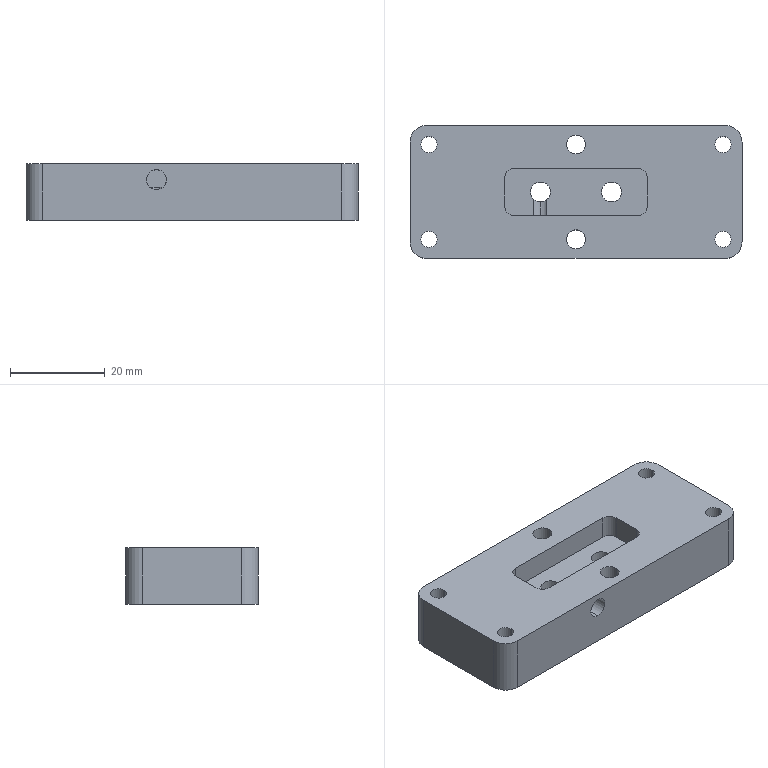Part | STEP file | 11-FG-SB01311 | 1 solid | 49 faces | box 70 x 28 x 12 mm | volume 20524 mm3 | cylinder 34 | plane 15 | commonest cylinder face diameters 3.4 x8 4 x8 6.5 x8 4.2 x6 7 x4
STEP:
#1=CARTESIAN_POINT('',(-7.5,-5.,10.7));
#2=VERTEX_POINT('',#1);
#3=CARTESIAN_POINT('',(-8.86,-5.,7.));
#4=VERTEX_POINT('',#3);
#5=CARTESIAN_POINT('',(-7.5,-5.,8.6));
#6=DIRECTION('',(0.,-1.,0.));
#7=DIRECTION('',(1.,0.,0.));
#8=AXIS2_PLACEMENT_3D('',#5,#6,#7);
#9=CIRCLE('',#8,2.1);
#10=EDGE_CURVE('',#2,#4,#9,.T.);
#11=ORIENTED_EDGE('',*,*,#10,.F.);
#12=CARTESIAN_POINT('',(-7.5,-14.,10.7));
#13=VERTEX_POINT('',#12);
#14=CARTESIAN_POINT('',(-7.5,-14.,10.7));
#15=DIRECTION('',(0.,-1.,0.));
#16=VECTOR('',#15,1000.);
#17=LINE('',#14,#16);
#18=EDGE_CURVE('',#2,#13,#17,.T.);
#19=ORIENTED_EDGE('',*,*,#18,.T.);
#20=CARTESIAN_POINT('',(-7.5,-14.,6.5));
#21=VERTEX_POINT('',#20);
#22=CARTESIAN_POINT('',(-7.5,-14.,8.6));
#23=DIRECTION('',(0.,-1.,0.));
#24=DIRECTION('',(0.,0.,-1.));
#25=AXIS2_PLACEMENT_3D('',#22,#23,#24);
#26=CIRCLE('',#25,2.1);
#27=EDGE_CURVE('',#13,#21,#26,.T.);
#28=ORIENTED_EDGE('',*,*,#27,.T.);
#29=CARTESIAN_POINT('',(-7.5,-2.1,6.5));
#30=VERTEX_POINT('',#29);
#31=CARTESIAN_POINT('',(-7.5,-14.,6.5));
#32=DIRECTION('',(0.,-1.,0.));
#33=VECTOR('',#32,1000.);
#34=LINE('',#31,#33);
#35=EDGE_CURVE('',#30,#21,#34,.T.);
#36=ORIENTED_EDGE('',*,*,#35,.F.);
#37=CARTESIAN_POINT('',(-8.86,-1.6,7.));
#38=VERTEX_POINT('',#37);
#39=CARTESIAN_POINT('',(-8.86,-1.6,7.));
#40=CARTESIAN_POINT('',(-8.476,-1.926,6.674));
#41=CARTESIAN_POINT('',(-8.004,-2.1,6.5));
#42=CARTESIAN_POINT('',(-7.5,-2.1,6.5));
#43=(BOUNDED_CURVE()B_SPLINE_CURVE(3,(#39,#40,#41,#42),.UNSPECIFIED.,.F.,.F.)B_SPLINE_CURVE_WITH_KNOTS((4,4),(2.437,3.142),.UNSPECIFIED.)CURVE()GEOMETRIC_REPRESENTATION_ITEM()RATIONAL_B_SPLINE_CURVE((1.,0.9591,0.9591,1.))REPRESENTATION_ITEM(''));
#44=EDGE_CURVE('',#38,#30,#43,.T.);
#45=ORIENTED_EDGE('',*,*,#44,.F.);
#46=CARTESIAN_POINT('',(-8.86,-14.,7.));
#47=DIRECTION('',(0.,1.,0.));
#48=VECTOR('',#47,1000.);
#49=LINE('',#46,#48);
#50=EDGE_CURVE('',#4,#38,#49,.T.);
#51=ORIENTED_EDGE('',*,*,#50,.F.);
#52=EDGE_LOOP('',(#11,#19,#28,#36,#45,#51));
#53=FACE_OUTER_BOUND('',#52,.T.);
#54=CARTESIAN_POINT('',(-7.5,-14.,8.6));
#55=DIRECTION('',(0.,-1.,0.));
#56=DIRECTION('',(0.,0.,-1.));
#57=AXIS2_PLACEMENT_3D('',#54,#55,#56);
#58=CYLINDRICAL_SURFACE('',#57,2.1);
#59=ADVANCED_FACE('',(#53),#58,.F.);
#60=CARTESIAN_POINT('',(-9.6,0.,0.));
#61=VERTEX_POINT('',#60);
#62=CARTESIAN_POINT('',(-5.4,0.,0.));
#63=VERTEX_POINT('',#62);
#64=CARTESIAN_POINT('',(-7.5,0.,0.));
#65=DIRECTION('',(0.,0.,1.));
#66=DIRECTION('',(1.,0.,0.));
#67=AXIS2_PLACEMENT_3D('',#64,#65,#66);
#68=CIRCLE('',#67,2.1);
#69=EDGE_CURVE('',#61,#63,#68,.T.);
#70=ORIENTED_EDGE('',*,*,#69,.F.);
#71=CARTESIAN_POINT('',(-9.6,0.,7.));
#72=VERTEX_POINT('',#71);
#73=CARTESIAN_POINT('',(-9.6,0.,7.));
#74=DIRECTION('',(0.,0.,1.));
#75=VECTOR('',#74,1000.);
#76=LINE('',#73,#75);
#77=EDGE_CURVE('',#61,#72,#76,.T.);
#78=ORIENTED_EDGE('',*,*,#77,.T.);
#79=CARTESIAN_POINT('',(-7.5,0.,7.));
#80=DIRECTION('',(0.,0.,1.));
#81=DIRECTION('',(1.,0.,0.));
#82=AXIS2_PLACEMENT_3D('',#79,#80,#81);
#83=CIRCLE('',#82,2.1);
#84=EDGE_CURVE('',#72,#38,#83,.T.);
#85=ORIENTED_EDGE('',*,*,#84,.T.);
#86=ORIENTED_EDGE('',*,*,#44,.T.);
#87=CARTESIAN_POINT('',(-6.14,-1.6,7.));
#88=VERTEX_POINT('',#87);
#89=CARTESIAN_POINT('',(-7.5,-2.1,6.5));
#90=CARTESIAN_POINT('',(-6.996,-2.1,6.5));
#91=CARTESIAN_POINT('',(-6.524,-1.926,6.674));
#92=CARTESIAN_POINT('',(-6.14,-1.6,7.));
#93=(BOUNDED_CURVE()B_SPLINE_CURVE(3,(#89,#90,#91,#92),.UNSPECIFIED.,.F.,.F.)B_SPLINE_CURVE_WITH_KNOTS((4,4),(3.142,3.846),.UNSPECIFIED.)CURVE()GEOMETRIC_REPRESENTATION_ITEM()RATIONAL_B_SPLINE_CURVE((1.,0.9591,0.9591,1.))REPRESENTATION_ITEM(''));
#94=EDGE_CURVE('',#30,#88,#93,.T.);
#95=ORIENTED_EDGE('',*,*,#94,.T.);
#96=CARTESIAN_POINT('',(-5.4,0.,7.));
#97=VERTEX_POINT('',#96);
#98=CARTESIAN_POINT('',(-7.5,0.,7.));
#99=DIRECTION('',(0.,0.,1.));
#100=DIRECTION('',(1.,0.,0.));
#101=AXIS2_PLACEMENT_3D('',#98,#99,#100);
#102=CIRCLE('',#101,2.1);
#103=EDGE_CURVE('',#88,#97,#102,.T.);
#104=ORIENTED_EDGE('',*,*,#103,.T.);
#105=CARTESIAN_POINT('',(-5.4,0.,7.));
#106=DIRECTION('',(0.,0.,1.));
#107=VECTOR('',#106,1000.);
#108=LINE('',#105,#107);
#109=EDGE_CURVE('',#63,#97,#108,.T.);
#110=ORIENTED_EDGE('',*,*,#109,.F.);
#111=EDGE_LOOP('',(#70,#78,#85,#86,#95,#104,#110));
#112=FACE_OUTER_BOUND('',#111,.T.);
#113=CARTESIAN_POINT('',(-7.5,0.,7.));
#114=DIRECTION('',(0.,0.,1.));
#115=DIRECTION('',(1.,0.,0.));
#116=AXIS2_PLACEMENT_3D('',#113,#114,#115);
#117=CYLINDRICAL_SURFACE('',#116,2.1);
#118=ADVANCED_FACE('',(#112),#117,.F.);
#119=CARTESIAN_POINT('',(5.4,0.,0.));
#120=VERTEX_POINT('',#119);
#121=CARTESIAN_POINT('',(9.6,0.,0.));
#122=VERTEX_POINT('',#121);
#123=CARTESIAN_POINT('',(7.5,0.,0.));
#124=DIRECTION('',(0.,0.,1.));
#125=DIRECTION('',(1.,0.,0.));
#126=AXIS2_PLACEMENT_3D('',#123,#124,#125);
#127=CIRCLE('',#126,2.1);
#128=EDGE_CURVE('',#120,#122,#127,.T.);
#129=ORIENTED_EDGE('',*,*,#128,.F.);
#130=CARTESIAN_POINT('',(5.4,0.,7.));
#131=VERTEX_POINT('',#130);
#132=CARTESIAN_POINT('',(5.4,0.,7.));
#133=DIRECTION('',(0.,0.,1.));
#134=VECTOR('',#133,1000.);
#135=LINE('',#132,#134);
#136=EDGE_CURVE('',#120,#131,#135,.T.);
#137=ORIENTED_EDGE('',*,*,#136,.T.);
#138=CARTESIAN_POINT('',(9.6,0.,7.));
#139=VERTEX_POINT('',#138);
#140=CARTESIAN_POINT('',(7.5,0.,7.));
#141=DIRECTION('',(0.,0.,1.));
#142=DIRECTION('',(1.,0.,0.));
#143=AXIS2_PLACEMENT_3D('',#140,#141,#142);
#144=CIRCLE('',#143,2.1);
#145=EDGE_CURVE('',#131,#139,#144,.T.);
#146=ORIENTED_EDGE('',*,*,#145,.T.);
#147=CARTESIAN_POINT('',(9.6,0.,7.));
#148=DIRECTION('',(0.,0.,1.));
#149=VECTOR('',#148,1000.);
#150=LINE('',#147,#149);
#151=EDGE_CURVE('',#122,#139,#150,.T.);
#152=ORIENTED_EDGE('',*,*,#151,.F.);
#153=EDGE_LOOP('',(#129,#137,#146,#152));
#154=FACE_OUTER_BOUND('',#153,.T.);
#155=CARTESIAN_POINT('',(7.5,0.,7.));
#156=DIRECTION('',(0.,0.,1.));
#157=DIRECTION('',(1.,0.,0.));
#158=AXIS2_PLACEMENT_3D('',#155,#156,#157);
#159=CYLINDRICAL_SURFACE('',#158,2.1);
#160=ADVANCED_FACE('',(#154),#159,.F.);
#161=CARTESIAN_POINT('',(-2.,10.,12.));
#162=VERTEX_POINT('',#161);
#163=CARTESIAN_POINT('',(2.,10.,12.));
#164=VERTEX_POINT('',#163);
#165=CARTESIAN_POINT('',(0.,10.,12.));
#166=DIRECTION('',(0.,0.,1.));
#167=DIRECTION('',(1.,0.,0.));
#168=AXIS2_PLACEMENT_3D('',#165,#166,#167);
#169=CIRCLE('',#168,2.);
#170=EDGE_CURVE('',#162,#164,#169,.T.);
#171=ORIENTED_EDGE('',*,*,#170,.T.);
#172=CARTESIAN_POINT('',(2.,10.,0.));
#173=VERTEX_POINT('',#172);
#174=CARTESIAN_POINT('',(2.,10.,0.));
#175=DIRECTION('',(0.,0.,-1.));
#176=VECTOR('',#175,1000.);
#177=LINE('',#174,#176);
#178=EDGE_CURVE('',#164,#173,#177,.T.);
#179=ORIENTED_EDGE('',*,*,#178,.T.);
#180=CARTESIAN_POINT('',(-2.,10.,0.));
#181=VERTEX_POINT('',#180);
#182=CARTESIAN_POINT('',(0.,10.,0.));
#183=DIRECTION('',(0.,0.,-1.));
#184=DIRECTION('',(-1.,0.,0.));
#185=AXIS2_PLACEMENT_3D('',#182,#183,#184);
#186=CIRCLE('',#185,2.);
#187=EDGE_CURVE('',#173,#181,#186,.T.);
#188=ORIENTED_EDGE('',*,*,#187,.T.);
#189=CARTESIAN_POINT('',(-2.,10.,0.));
#190=DIRECTION('',(0.,0.,-1.));
#191=VECTOR('',#190,1000.);
#192=LINE('',#189,#191);
#193=EDGE_CURVE('',#162,#181,#192,.T.);
#194=ORIENTED_EDGE('',*,*,#193,.F.);
#195=EDGE_LOOP('',(#171,#179,#188,#194));
#196=FACE_OUTER_BOUND('',#195,.T.);
#197=CARTESIAN_POINT('',(0.,10.,0.));
#198=DIRECTION('',(0.,0.,-1.));
#199=DIRECTION('',(-1.,0.,0.));
#200=AXIS2_PLACEMENT_3D('',#197,#198,#199);
#201=CYLINDRICAL_SURFACE('',#200,2.);
#202=ADVANCED_FACE('',(#196),#201,.F.);
#203=CARTESIAN_POINT('',(-2.,-10.,12.));
#204=VERTEX_POINT('',#203);
#205=CARTESIAN_POINT('',(2.,-10.,12.));
#206=VERTEX_POINT('',#205);
#207=CARTESIAN_POINT('',(0.,-10.,12.));
#208=DIRECTION('',(0.,0.,1.));
#209=DIRECTION('',(1.,0.,0.));
#210=AXIS2_PLACEMENT_3D('',#207,#208,#209);
#211=CIRCLE('',#210,2.);
#212=EDGE_CURVE('',#204,#206,#211,.T.);
#213=ORIENTED_EDGE('',*,*,#212,.T.);
#214=CARTESIAN_POINT('',(2.,-10.,0.));
#215=VERTEX_POINT('',#214);
#216=CARTESIAN_POINT('',(2.,-10.,0.));
#217=DIRECTION('',(0.,0.,-1.));
#218=VECTOR('',#217,1000.);
#219=LINE('',#216,#218);
#220=EDGE_CURVE('',#206,#215,#219,.T.);
#221=ORIENTED_EDGE('',*,*,#220,.T.);
#222=CARTESIAN_POINT('',(-2.,-10.,0.));
#223=VERTEX_POINT('',#222);
#224=CARTESIAN_POINT('',(0.,-10.,0.));
#225=DIRECTION('',(0.,0.,-1.));
#226=DIRECTION('',(-1.,0.,0.));
#227=AXIS2_PLACEMENT_3D('',#224,#225,#226);
#228=CIRCLE('',#227,2.);
#229=EDGE_CURVE('',#215,#223,#228,.T.);
#230=ORIENTED_EDGE('',*,*,#229,.T.);
#231=CARTESIAN_POINT('',(-2.,-10.,0.));
#232=DIRECTION('',(0.,0.,-1.));
#233=VECTOR('',#232,1000.);
#234=LINE('',#231,#233);
#235=EDGE_CURVE('',#204,#223,#234,.T.);
#236=ORIENTED_EDGE('',*,*,#235,.F.);
#237=EDGE_LOOP('',(#213,#221,#230,#236));
#238=FACE_OUTER_BOUND('',#237,.T.);
#239=CARTESIAN_POINT('',(0.,-10.,0.));
#240=DIRECTION('',(0.,0.,-1.));
#241=DIRECTION('',(-1.,0.,0.));
#242=AXIS2_PLACEMENT_3D('',#239,#240,#241);
#243=CYLINDRICAL_SURFACE('',#242,2.);
#244=ADVANCED_FACE('',(#238),#243,.F.);
#245=CARTESIAN_POINT('',(34.25,10.,3.4));
#246=VERTEX_POINT('',#245);
#247=CARTESIAN_POINT('',(27.75,10.,3.4));
#248=VERTEX_POINT('',#247);
#249=CARTESIAN_POINT('',(31.,10.,3.4));
#250=DIRECTION('',(0.,0.,-1.));
#251=DIRECTION('',(-1.,0.,0.));
#252=AXIS2_PLACEMENT_3D('',#249,#250,#251);
#253=CIRCLE('',#252,3.25);
#254=EDGE_CURVE('',#246,#248,#253,.T.);
#255=ORIENTED_EDGE('',*,*,#254,.F.);
#256=CARTESIAN_POINT('',(34.25,10.,0.));
#257=VERTEX_POINT('',#256);
#258=CARTESIAN_POINT('',(34.25,10.,0.));
#259=DIRECTION('',(0.,0.,-1.));
#260=VECTOR('',#259,1000.);
#261=LINE('',#258,#260);
#262=EDGE_CURVE('',#246,#257,#261,.T.);
#263=ORIENTED_EDGE('',*,*,#262,.T.);
#264=CARTESIAN_POINT('',(27.75,10.,0.));
#265=VERTEX_POINT('',#264);
#266=CARTESIAN_POINT('',(31.,10.,0.));
#267=DIRECTION('',(0.,0.,-1.));
#268=DIRECTION('',(-1.,0.,0.));
#269=AXIS2_PLACEMENT_3D('',#266,#267,#268);
#270=CIRCLE('',#269,3.25);
#271=EDGE_CURVE('',#257,#265,#270,.T.);
#272=ORIENTED_EDGE('',*,*,#271,.T.);
#273=CARTESIAN_POINT('',(27.75,10.,0.));
#274=DIRECTION('',(0.,0.,-1.));
#275=VECTOR('',#274,1000.);
#276=LINE('',#273,#275);
#277=EDGE_CURVE('',#248,#265,#276,.T.);
#278=ORIENTED_EDGE('',*,*,#277,.F.);
#279=EDGE_LOOP('',(#255,#263,#272,#278));
#280=FACE_OUTER_BOUND('',#279,.T.);
#281=CARTESIAN_POINT('',(31.,10.,0.));
#282=DIRECTION('',(0.,0.,-1.));
#283=DIRECTION('',(-1.,0.,0.));
#284=AXIS2_PLACEMENT_3D('',#281,#282,#283);
#285=CYLINDRICAL_SURFACE('',#284,3.25);
#286=ADVANCED_FACE('',(#280),#285,.F.);
#287=CARTESIAN_POINT('',(29.3,10.,12.));
#288=VERTEX_POINT('',#287);
#289=CARTESIAN_POINT('',(32.7,10.,12.));
#290=VERTEX_POINT('',#289);
#291=CARTESIAN_POINT('',(31.,10.,12.));
#292=DIRECTION('',(0.,0.,1.));
#293=DIRECTION('',(1.,0.,0.));
#294=AXIS2_PLACEMENT_3D('',#291,#292,#293);
#295=CIRCLE('',#294,1.7);
#296=EDGE_CURVE('',#288,#290,#295,.T.);
#297=ORIENTED_EDGE('',*,*,#296,.T.);
#298=CARTESIAN_POINT('',(32.7,10.,3.4));
#299=VERTEX_POINT('',#298);
#300=CARTESIAN_POINT('',(32.7,10.,0.));
#301=DIRECTION('',(0.,0.,-1.));
#302=VECTOR('',#301,1000.);
#303=LINE('',#300,#302);
#304=EDGE_CURVE('',#290,#299,#303,.T.);
#305=ORIENTED_EDGE('',*,*,#304,.T.);
#306=CARTESIAN_POINT('',(29.3,10.,3.4));
#307=VERTEX_POINT('',#306);
#308=CARTESIAN_POINT('',(31.,10.,3.4));
#309=DIRECTION('',(0.,0.,-1.));
#310=DIRECTION('',(-1.,0.,0.));
#311=AXIS2_PLACEMENT_3D('',#308,#309,#310);
#312=CIRCLE('',#311,1.7);
#313=EDGE_CURVE('',#299,#307,#312,.T.);
#314=ORIENTED_EDGE('',*,*,#313,.T.);
#315=CARTESIAN_POINT('',(29.3,10.,0.));
#316=DIRECTION('',(0.,0.,-1.));
#317=VECTOR('',#316,1000.);
#318=LINE('',#315,#317);
#319=EDGE_CURVE('',#288,#307,#318,.T.);
#320=ORIENTED_EDGE('',*,*,#319,.F.);
#321=EDGE_LOOP('',(#297,#305,#314,#320));
#322=FACE_OUTER_BOUND('',#321,.T.);
#323=CARTESIAN_POINT('',(31.,10.,0.));
#324=DIRECTION('',(0.,0.,-1.));
#325=DIRECTION('',(-1.,0.,0.));
#326=AXIS2_PLACEMENT_3D('',#323,#324,#325);
#327=CYLINDRICAL_SURFACE('',#326,1.7);
#328=ADVANCED_FACE('',(#322),#327,.F.);
#329=CARTESIAN_POINT('',(-27.75,10.,3.4));
#330=VERTEX_POINT('',#329);
#331=CARTESIAN_POINT('',(-34.25,10.,3.4));
#332=VERTEX_POINT('',#331);
#333=CARTESIAN_POINT('',(-31.,10.,3.4));
#334=DIRECTION('',(0.,0.,-1.));
#335=DIRECTION('',(-1.,0.,0.));
#336=AXIS2_PLACEMENT_3D('',#333,#334,#335);
#337=CIRCLE('',#336,3.25);
#338=EDGE_CURVE('',#330,#332,#337,.T.);
#339=ORIENTED_EDGE('',*,*,#338,.F.);
#340=CARTESIAN_POINT('',(-27.75,10.,0.));
#341=VERTEX_POINT('',#340);
#342=CARTESIAN_POINT('',(-27.75,10.,0.));
#343=DIRECTION('',(0.,0.,-1.));
#344=VECTOR('',#343,1000.);
#345=LINE('',#342,#344);
#346=EDGE_CURVE('',#330,#341,#345,.T.);
#347=ORIENTED_EDGE('',*,*,#346,.T.);
#348=CARTESIAN_POINT('',(-34.25,10.,0.));
#349=VERTEX_POINT('',#348);
#350=CARTESIAN_POINT('',(-31.,10.,0.));
#351=DIRECTION('',(0.,0.,-1.));
#352=DIRECTION('',(-1.,0.,0.));
#353=AXIS2_PLACEMENT_3D('',#350,#351,#352);
#354=CIRCLE('',#353,3.25);
#355=EDGE_CURVE('',#341,#349,#354,.T.);
#356=ORIENTED_EDGE('',*,*,#355,.T.);
#357=CARTESIAN_POINT('',(-34.25,10.,0.));
#358=DIRECTION('',(0.,0.,-1.));
#359=VECTOR('',#358,1000.);
#360=LINE('',#357,#359);
#361=EDGE_CURVE('',#332,#349,#360,.T.);
#362=ORIENTED_EDGE('',*,*,#361,.F.);
#363=EDGE_LOOP('',(#339,#347,#356,#362));
#364=FACE_OUTER_BOUND('',#363,.T.);
#365=CARTESIAN_POINT('',(-31.,10.,0.));
#366=DIRECTION('',(0.,0.,-1.));
#367=DIRECTION('',(-1.,0.,0.));
#368=AXIS2_PLACEMENT_3D('',#365,#366,#367);
#369=CYLINDRICAL_SURFACE('',#368,3.25);
#370=ADVANCED_FACE('',(#364),#369,.F.);
#371=CARTESIAN_POINT('',(-32.7,10.,12.));
#372=VERTEX_POINT('',#371);
#373=CARTESIAN_POINT('',(-29.3,10.,12.));
#374=VERTEX_POINT('',#373);
#375=CARTESIAN_POINT('',(-31.,10.,12.));
#376=DIRECTION('',(0.,0.,1.));
#377=DIRECTION('',(1.,0.,0.));
#378=AXIS2_PLACEMENT_3D('',#375,#376,#377);
#379=CIRCLE('',#378,1.7);
#380=EDGE_CURVE('',#372,#374,#379,.T.);
#381=ORIENTED_EDGE('',*,*,#380,.T.);
#382=CARTESIAN_POINT('',(-29.3,10.,3.4));
#383=VERTEX_POINT('',#382);
#384=CARTESIAN_POINT('',(-29.3,10.,0.));
#385=DIRECTION('',(0.,0.,-1.));
#386=VECTOR('',#385,1000.);
#387=LINE('',#384,#386);
#388=EDGE_CURVE('',#374,#383,#387,.T.);
#389=ORIENTED_EDGE('',*,*,#388,.T.);
#390=CARTESIAN_POINT('',(-32.7,10.,3.4));
#391=VERTEX_POINT('',#390);
#392=CARTESIAN_POINT('',(-31.,10.,3.4));
#393=DIRECTION('',(0.,0.,-1.));
#394=DIRECTION('',(-1.,0.,0.));
#395=AXIS2_PLACEMENT_3D('',#392,#393,#394);
#396=CIRCLE('',#395,1.7);
#397=EDGE_CURVE('',#383,#391,#396,.T.);
#398=ORIENTED_EDGE('',*,*,#397,.T.);
#399=CARTESIAN_POINT('',(-32.7,10.,0.));
#400=DIRECTION('',(0.,0.,-1.));
#401=VECTOR('',#400,1000.);
#402=LINE('',#399,#401);
#403=EDGE_CURVE('',#372,#391,#402,.T.);
#404=ORIENTED_EDGE('',*,*,#403,.F.);
#405=EDGE_LOOP('',(#381,#389,#398,#404));
#406=FACE_OUTER_BOUND('',#405,.T.);
#407=CARTESIAN_POINT('',(-31.,10.,0.));
#408=DIRECTION('',(0.,0.,-1.));
#409=DIRECTION('',(-1.,0.,0.));
#410=AXIS2_PLACEMENT_3D('',#407,#408,#409);
#411=CYLINDRICAL_SURFACE('',#410,1.7);
#412=ADVANCED_FACE('',(#406),#411,.F.);
#413=CARTESIAN_POINT('',(34.25,-10.,3.4));
#414=VERTEX_POINT('',#413);
#415=CARTESIAN_POINT('',(27.75,-10.,3.4));
#416=VERTEX_POINT('',#415);
#417=CARTESIAN_POINT('',(31.,-10.,3.4));
#418=DIRECTION('',(0.,0.,-1.));
#419=DIRECTION('',(-1.,0.,0.));
#420=AXIS2_PLACEMENT_3D('',#417,#418,#419);
#421=CIRCLE('',#420,3.25);
#422=EDGE_CURVE('',#414,#416,#421,.T.);
#423=ORIENTED_EDGE('',*,*,#422,.F.);
#424=CARTESIAN_POINT('',(34.25,-10.,0.));
#425=VERTEX_POINT('',#424);
#426=CARTESIAN_POINT('',(34.25,-10.,0.));
#427=DIRECTION('',(0.,0.,-1.));
#428=VECTOR('',#427,1000.);
#429=LINE('',#426,#428);
#430=EDGE_CURVE('',#414,#425,#429,.T.);
#431=ORIENTED_EDGE('',*,*,#430,.T.);
#432=CARTESIAN_POINT('',(27.75,-10.,0.));
#433=VERTEX_POINT('',#432);
#434=CARTESIAN_POINT('',(31.,-10.,0.));
#435=DIRECTION('',(0.,0.,-1.));
#436=DIRECTION('',(-1.,0.,0.));
#437=AXIS2_PLACEMENT_3D('',#434,#435,#436);
#438=CIRCLE('',#437,3.25);
#439=EDGE_CURVE('',#425,#433,#438,.T.);
#440=ORIENTED_EDGE('',*,*,#439,.T.);
#441=CARTESIAN_POINT('',(27.75,-10.,0.));
#442=DIRECTION('',(0.,0.,-1.));
#443=VECTOR('',#442,1000.);
#444=LINE('',#441,#443);
#445=EDGE_CURVE('',#416,#433,#444,.T.);
#446=ORIENTED_EDGE('',*,*,#445,.F.);
#447=EDGE_LOOP('',(#423,#431,#440,#446));
#448=FACE_OUTER_BOUND('',#447,.T.);
#449=CARTESIAN_POINT('',(31.,-10.,0.));
#450=DIRECTION('',(0.,0.,-1.));
#451=DIRECTION('',(-1.,0.,0.));
#452=AXIS2_PLACEMENT_3D('',#449,#450,#451);
#453=CYLINDRICAL_SURFACE('',#452,3.25);
#454=ADVANCED_FACE('',(#448),#453,.F.);
#455=CARTESIAN_POINT('',(29.3,-10.,12.));
#456=VERTEX_POINT('',#455);
#457=CARTESIAN_POINT('',(32.7,-10.,12.));
#458=VERTEX_POINT('',#457);
#459=CARTESIAN_POINT('',(31.,-10.,12.));
#460=DIRECTION('',(0.,0.,1.));
#461=DIRECTION('',(1.,0.,0.));
#462=AXIS2_PLACEMENT_3D('',#459,#460,#461);
#463=CIRCLE('',#462,1.7);
#464=EDGE_CURVE('',#456,#458,#463,.T.);
#465=ORIENTED_EDGE('',*,*,#464,.T.);
#466=CARTESIAN_POINT('',(32.7,-10.,3.4));
#467=VERTEX_POINT('',#466);
#468=CARTESIAN_POINT('',(32.7,-10.,0.));
#469=DIRECTION('',(0.,0.,-1.));
#470=VECTOR('',#469,1000.);
#471=LINE('',#468,#470);
#472=EDGE_CURVE('',#458,#467,#471,.T.);
#473=ORIENTED_EDGE('',*,*,#472,.T.);
#474=CARTESIAN_POINT('',(29.3,-10.,3.4));
#475=VERTEX_POINT('',#474);
#476=CARTESIAN_POINT('',(31.,-10.,3.4));
#477=DIRECTION('',(0.,0.,-1.));
#478=DIRECTION('',(-1.,0.,0.));
#479=AXIS2_PLACEMENT_3D('',#476,#477,#478);
#480=CIRCLE('',#479,1.7);
#481=EDGE_CURVE('',#467,#475,#480,.T.);
#482=ORIENTED_EDGE('',*,*,#481,.T.);
#483=CARTESIAN_POINT('',(29.3,-10.,0.));
#484=DIRECTION('',(0.,0.,-1.));
#485=VECTOR('',#484,1000.);
#486=LINE('',#483,#485);
#487=EDGE_CURVE('',#456,#475,#486,.T.);
#488=ORIENTED_EDGE('',*,*,#487,.F.);
#489=EDGE_LOOP('',(#465,#473,#482,#488));
#490=FACE_OUTER_BOUND('',#489,.T.);
#491=CARTESIAN_POINT('',(31.,-10.,0.));
#492=DIRECTION('',(0.,0.,-1.));
#493=DIRECTION('',(-1.,0.,0.));
#494=AXIS2_PLACEMENT_3D('',#491,#492,#493);
#495=CYLINDRICAL_SURFACE('',#494,1.7);
#496=ADVANCED_FACE('',(#490),#495,.F.);
#497=CARTESIAN_POINT('',(-27.75,-10.,3.4));
#498=VERTEX_POINT('',#497);
#499=CARTESIAN_POINT('',(-34.25,-10.,3.4));
#500=VERTEX_POINT('',#499);
#501=CARTESIAN_POINT('',(-31.,-10.,3.4));
#502=DIRECTION('',(0.,0.,-1.));
#503=DIRECTION('',(-1.,0.,0.));
#504=AXIS2_PLACEMENT_3D('',#501,#502,#503);
#505=CIRCLE('',#504,3.25);
#506=EDGE_CURVE('',#498,#500,#505,.T.);
#507=ORIENTED_EDGE('',*,*,#506,.F.);
#508=CARTESIAN_POINT('',(-27.75,-10.,0.));
#509=VERTEX_POINT('',#508);
#510=CARTESIAN_POINT('',(-27.75,-10.,0.));
#511=DIRECTION('',(0.,0.,-1.));
#512=VECTOR('',#511,1000.);
#513=LINE('',#510,#512);
#514=EDGE_CURVE('',#498,#509,#513,.T.);
#515=ORIENTED_EDGE('',*,*,#514,.T.);
#516=CARTESIAN_POINT('',(-34.25,-10.,0.));
#517=VERTEX_POINT('',#516);
#518=CARTESIAN_POINT('',(-31.,-10.,0.));
#519=DIRECTION('',(0.,0.,-1.));
#520=DIRECTION('',(-1.,0.,0.));
#521=AXIS2_PLACEMENT_3D('',#518,#519,#520);
#522=CIRCLE('',#521,3.25);
#523=EDGE_CURVE('',#509,#517,#522,.T.);
#524=ORIENTED_EDGE('',*,*,#523,.T.);
#525=CARTESIAN_POINT('',(-34.25,-10.,0.));
#526=DIRECTION('',(0.,0.,-1.));
#527=VECTOR('',#526,1000.);
#528=LINE('',#525,#527);
#529=EDGE_CURVE('',#500,#517,#528,.T.);
#530=ORIENTED_EDGE('',*,*,#529,.F.);
#531=EDGE_LOOP('',(#507,#515,#524,#530));
#532=FACE_OUTER_BOUND('',#531,.T.);
#533=CARTESIAN_POINT('',(-31.,-10.,0.));
#534=DIRECTION('',(0.,0.,-1.));
#535=DIRECTION('',(-1.,0.,0.));
#536=AXIS2_PLACEMENT_3D('',#533,#534,#535);
#537=CYLINDRICAL_SURFACE('',#536,3.25);
#538=ADVANCED_FACE('',(#532),#537,.F.);
#539=CARTESIAN_POINT('',(-32.7,-10.,12.));
#540=VERTEX_POINT('',#539);
#541=CARTESIAN_POINT('',(-29.3,-10.,12.));
#542=VERTEX_POINT('',#541);
#543=CARTESIAN_POINT('',(-31.,-10.,12.));
#544=DIRECTION('',(0.,0.,1.));
#545=DIRECTION('',(1.,0.,0.));
#546=AXIS2_PLACEMENT_3D('',#543,#544,#545);
#547=CIRCLE('',#546,1.7);
#548=EDGE_CURVE('',#540,#542,#547,.T.);
#549=ORIENTED_EDGE('',*,*,#548,.T.);
#550=CARTESIAN_POINT('',(-29.3,-10.,3.4));
#551=VERTEX_POINT('',#550);
#552=CARTESIAN_POINT('',(-29.3,-10.,0.));
#553=DIRECTION('',(0.,0.,-1.));
#554=VECTOR('',#553,1000.);
#555=LINE('',#552,#554);
#556=EDGE_CURVE('',#542,#551,#555,.T.);
#557=ORIENTED_EDGE('',*,*,#556,.T.);
#558=CARTESIAN_POINT('',(-32.7,-10.,3.4));
#559=VERTEX_POINT('',#558);
#560=CARTESIAN_POINT('',(-31.,-10.,3.4));
#561=DIRECTION('',(0.,0.,-1.));
#562=DIRECTION('',(-1.,0.,0.));
#563=AXIS2_PLACEMENT_3D('',#560,#561,#562);
#564=CIRCLE('',#563,1.7);
#565=EDGE_CURVE('',#551,#559,#564,.T.);
#566=ORIENTED_EDGE('',*,*,#565,.T.);
#567=CARTESIAN_POINT('',(-32.7,-10.,0.));
#568=DIRECTION('',(0.,0.,-1.));
#569=VECTOR('',#568,1000.);
#570=LINE('',#567,#569);
#571=EDGE_CURVE('',#540,#559,#570,.T.);
#572=ORIENTED_EDGE('',*,*,#571,.F.);
#573=EDGE_LOOP('',(#549,#557,#566,#572));
#574=FACE_OUTER_BOUND('',#573,.T.);
#575=CARTESIAN_POINT('',(-31.,-10.,0.));
#576=DIRECTION('',(0.,0.,-1.));
#577=DIRECTION('',(-1.,0.,0.));
#578=AXIS2_PLACEMENT_3D('',#575,#576,#577);
#579=CYLINDRICAL_SURFACE('',#578,1.7);
#580=ADVANCED_FACE('',(#574),#579,.F.);
#581=CARTESIAN_POINT('',(-7.5,0.,0.));
#582=DIRECTION('',(0.,0.,1.));
#583=DIRECTION('',(1.,0.,0.));
#584=AXIS2_PLACEMENT_3D('',#581,#582,#583);
#585=CIRCLE('',#584,2.1);
#586=EDGE_CURVE('',#63,#61,#585,.T.);
#587=ORIENTED_EDGE('',*,*,#586,.T.);
#588=ORIENTED_EDGE('',*,*,#69,.T.);
#589=EDGE_LOOP('',(#587,#588));
#590=FACE_BOUND('',#589,.T.);
#591=CARTESIAN_POINT('',(7.5,0.,0.));
#592=DIRECTION('',(0.,0.,1.));
#593=DIRECTION('',(1.,0.,0.));
#594=AXIS2_PLACEMENT_3D('',#591,#592,#593);
#595=CIRCLE('',#594,2.1);
#596=EDGE_CURVE('',#122,#120,#595,.T.);
#597=ORIENTED_EDGE('',*,*,#596,.T.);
#598=ORIENTED_EDGE('',*,*,#128,.T.);
#599=EDGE_LOOP('',(#597,#598));
#600=FACE_BOUND('',#599,.T.);
#601=CARTESIAN_POINT('',(31.,-10.,0.));
#602=DIRECTION('',(0.,0.,-1.));
#603=DIRECTION('',(-1.,0.,0.));
#604=AXIS2_PLACEMENT_3D('',#601,#602,#603);
#605=CIRCLE('',#604,3.25);
#606=EDGE_CURVE('',#433,#425,#605,.T.);
#607=ORIENTED_EDGE('',*,*,#606,.F.);
#608=ORIENTED_EDGE('',*,*,#439,.F.);
#609=EDGE_LOOP('',(#607,#608));
#610=FACE_BOUND('',#609,.T.);
#611=CARTESIAN_POINT('',(31.,10.,0.));
#612=DIRECTION('',(0.,0.,-1.));
#613=DIRECTION('',(-1.,0.,0.));
#614=AXIS2_PLACEMENT_3D('',#611,#612,#613);
#615=CIRCLE('',#614,3.25);
#616=EDGE_CURVE('',#265,#257,#615,.T.);
#617=ORIENTED_EDGE('',*,*,#616,.F.);
#618=ORIENTED_EDGE('',*,*,#271,.F.);
#619=EDGE_LOOP('',(#617,#618));
#620=FACE_BOUND('',#619,.T.);
#621=CARTESIAN_POINT('',(35.,-10.5,0.));
#622=VERTEX_POINT('',#621);
#623=CARTESIAN_POINT('',(31.5,-14.,0.));
#624=VERTEX_POINT('',#623);
#625=CARTESIAN_POINT('',(31.5,-10.5,0.));
#626=DIRECTION('',(0.,0.,-1.));
#627=DIRECTION('',(1.,0.,0.));
#628=AXIS2_PLACEMENT_3D('',#625,#626,#627);
#629=CIRCLE('',#628,3.5);
#630=EDGE_CURVE('',#622,#624,#629,.T.);
#631=ORIENTED_EDGE('',*,*,#630,.T.);
#632=CARTESIAN_POINT('',(-31.5,-14.,0.));
#633=VERTEX_POINT('',#632);
#634=CARTESIAN_POINT('',(-35.,-14.,0.));
#635=DIRECTION('',(1.,0.,0.));
#636=VECTOR('',#635,1000.);
#637=LINE('',#634,#636);
#638=EDGE_CURVE('',#633,#624,#637,.T.);
#639=ORIENTED_EDGE('',*,*,#638,.F.);
#640=CARTESIAN_POINT('',(-35.,-10.5,0.));
#641=VERTEX_POINT('',#640);
#642=CARTESIAN_POINT('',(-31.5,-10.5,0.));
#643=DIRECTION('',(0.,0.,-1.));
#644=DIRECTION('',(1.,0.,0.));
#645=AXIS2_PLACEMENT_3D('',#642,#643,#644);
#646=CIRCLE('',#645,3.5);
#647=EDGE_CURVE('',#633,#641,#646,.T.);
#648=ORIENTED_EDGE('',*,*,#647,.T.);
#649=CARTESIAN_POINT('',(-35.,10.5,0.));
#650=VERTEX_POINT('',#649);
#651=CARTESIAN_POINT('',(-35.,14.,0.));
#652=DIRECTION('',(0.,-1.,0.));
#653=VECTOR('',#652,1000.);
#654=LINE('',#651,#653);
#655=EDGE_CURVE('',#650,#641,#654,.T.);
#656=ORIENTED_EDGE('',*,*,#655,.F.);
#657=CARTESIAN_POINT('',(-31.5,14.,0.));
#658=VERTEX_POINT('',#657);
#659=CARTESIAN_POINT('',(-31.5,10.5,0.));
#660=DIRECTION('',(0.,0.,-1.));
#661=DIRECTION('',(1.,0.,0.));
#662=AXIS2_PLACEMENT_3D('',#659,#660,#661);
#663=CIRCLE('',#662,3.5);
#664=EDGE_CURVE('',#650,#658,#663,.T.);
#665=ORIENTED_EDGE('',*,*,#664,.T.);
#666=CARTESIAN_POINT('',(31.5,14.,0.));
#667=VERTEX_POINT('',#666);
#668=CARTESIAN_POINT('',(-35.,14.,0.));
#669=DIRECTION('',(-1.,0.,0.));
#670=VECTOR('',#669,1000.);
#671=LINE('',#668,#670);
#672=EDGE_CURVE('',#667,#658,#671,.T.);
#673=ORIENTED_EDGE('',*,*,#672,.F.);
#674=CARTESIAN_POINT('',(35.,10.5,0.));
#675=VERTEX_POINT('',#674);
#676=CARTESIAN_POINT('',(31.5,10.5,0.));
#677=DIRECTION('',(0.,0.,-1.));
#678=DIRECTION('',(1.,0.,0.));
#679=AXIS2_PLACEMENT_3D('',#676,#677,#678);
#680=CIRCLE('',#679,3.5);
#681=EDGE_CURVE('',#667,#675,#680,.T.);
#682=ORIENTED_EDGE('',*,*,#681,.T.);
#683=CARTESIAN_POINT('',(35.,14.,0.));
#684=DIRECTION('',(0.,1.,0.));
#685=VECTOR('',#684,1000.);
#686=LINE('',#683,#685);
#687=EDGE_CURVE('',#622,#675,#686,.T.);
#688=ORIENTED_EDGE('',*,*,#687,.F.);
#689=EDGE_LOOP('',(#631,#639,#648,#656,#665,#673,#682,#688));
#690=FACE_OUTER_BOUND('',#689,.T.);
#691=CARTESIAN_POINT('',(0.,10.,0.));
#692=DIRECTION('',(0.,0.,-1.));
#693=DIRECTION('',(-1.,0.,0.));
#694=AXIS2_PLACEMENT_3D('',#691,#692,#693);
#695=CIRCLE('',#694,2.);
#696=EDGE_CURVE('',#181,#173,#695,.T.);
#697=ORIENTED_EDGE('',*,*,#696,.F.);
#698=ORIENTED_EDGE('',*,*,#187,.F.);
#699=EDGE_LOOP('',(#697,#698));
#700=FACE_BOUND('',#699,.T.);
#701=CARTESIAN_POINT('',(0.,-10.,0.));
#702=DIRECTION('',(0.,0.,-1.));
#703=DIRECTION('',(-1.,0.,0.));
#704=AXIS2_PLACEMENT_3D('',#701,#702,#703);
#705=CIRCLE('',#704,2.);
#706=EDGE_CURVE('',#223,#215,#705,.T.);
#707=ORIENTED_EDGE('',*,*,#706,.F.);
#708=ORIENTED_EDGE('',*,*,#229,.F.);
#709=EDGE_LOOP('',(#707,#708));
#710=FACE_BOUND('',#709,.T.);
#711=CARTESIAN_POINT('',(-31.,10.,0.));
#712=DIRECTION('',(0.,0.,-1.));
#713=DIRECTION('',(-1.,0.,0.));
#714=AXIS2_PLACEMENT_3D('',#711,#712,#713);
#715=CIRCLE('',#714,3.25);
#716=EDGE_CURVE('',#349,#341,#715,.T.);
#717=ORIENTED_EDGE('',*,*,#716,.F.);
#718=ORIENTED_EDGE('',*,*,#355,.F.);
#719=EDGE_LOOP('',(#717,#718));
#720=FACE_BOUND('',#719,.T.);
#721=CARTESIAN_POINT('',(-31.,-10.,0.));
#722=DIRECTION('',(0.,0.,-1.));
#723=DIRECTION('',(-1.,0.,0.));
#724=AXIS2_PLACEMENT_3D('',#721,#722,#723);
#725=CIRCLE('',#724,3.25);
#726=EDGE_CURVE('',#517,#509,#725,.T.);
#727=ORIENTED_EDGE('',*,*,#726,.F.);
#728=ORIENTED_EDGE('',*,*,#523,.F.);
#729=EDGE_LOOP('',(#727,#728));
#730=FACE_BOUND('',#729,.T.);
#731=CARTESIAN_POINT('',(0.,0.,0.));
#732=DIRECTION('',(0.,0.,1.));
#733=DIRECTION('',(1.,0.,0.));
#734=AXIS2_PLACEMENT_3D('',#731,#732,#733);
#735=PLANE('',#734);
#736=ADVANCED_FACE('',(#590,#600,#610,#620,#690,#700,#710,#720,#730),#735,.F.);
#737=CARTESIAN_POINT('',(35.,-10.5,12.));
#738=VERTEX_POINT('',#737);
#739=CARTESIAN_POINT('',(35.,10.5,12.));
#740=VERTEX_POINT('',#739);
#741=CARTESIAN_POINT('',(35.,14.,12.));
#742=DIRECTION('',(0.,1.,0.));
#743=VECTOR('',#742,1000.);
#744=LINE('',#741,#743);
#745=EDGE_CURVE('',#738,#740,#744,.T.);
#746=ORIENTED_EDGE('',*,*,#745,.F.);
#747=CARTESIAN_POINT('',(35.,-10.5,12.));
#748=DIRECTION('',(0.,0.,-1.));
#749=VECTOR('',#748,1000.);
#750=LINE('',#747,#749);
#751=EDGE_CURVE('',#738,#622,#750,.T.);
#752=ORIENTED_EDGE('',*,*,#751,.T.);
#753=ORIENTED_EDGE('',*,*,#687,.T.);
#754=CARTESIAN_POINT('',(35.,10.5,12.));
#755=DIRECTION('',(0.,0.,1.));
#756=VECTOR('',#755,1000.);
#757=LINE('',#754,#756);
#758=EDGE_CURVE('',#675,#740,#757,.T.);
#759=ORIENTED_EDGE('',*,*,#758,.T.);
#760=EDGE_LOOP('',(#746,#752,#753,#759));
#761=FACE_OUTER_BOUND('',#760,.T.);
#762=CARTESIAN_POINT('',(35.,14.,12.));
#763=DIRECTION('',(-1.,0.,0.));
#764=DIRECTION('',(0.,0.,1.));
#765=AXIS2_PLACEMENT_3D('',#762,#763,#764);
#766=PLANE('',#765);
#767=ADVANCED_FACE('',(#761),#766,.F.);
#768=ORIENTED_EDGE('',*,*,#672,.T.);
#769=CARTESIAN_POINT('',(-31.5,14.,12.));
#770=VERTEX_POINT('',#769);
#771=CARTESIAN_POINT('',(-31.5,14.,12.));
#772=DIRECTION('',(0.,0.,1.));
#773=VECTOR('',#772,1000.);
#774=LINE('',#771,#773);
#775=EDGE_CURVE('',#658,#770,#774,.T.);
#776=ORIENTED_EDGE('',*,*,#775,.T.);
#777=CARTESIAN_POINT('',(31.5,14.,12.));
#778=VERTEX_POINT('',#777);
#779=CARTESIAN_POINT('',(-35.,14.,12.));
#780=DIRECTION('',(-1.,0.,0.));
#781=VECTOR('',#780,1000.);
#782=LINE('',#779,#781);
#783=EDGE_CURVE('',#778,#770,#782,.T.);
#784=ORIENTED_EDGE('',*,*,#783,.F.);
#785=CARTESIAN_POINT('',(31.5,14.,12.));
#786=DIRECTION('',(0.,0.,-1.));
#787=VECTOR('',#786,1000.);
#788=LINE('',#785,#787);
#789=EDGE_CURVE('',#778,#667,#788,.T.);
#790=ORIENTED_EDGE('',*,*,#789,.T.);
#791=EDGE_LOOP('',(#768,#776,#784,#790));
#792=FACE_OUTER_BOUND('',#791,.T.);
#793=CARTESIAN_POINT('',(-35.,14.,12.));
#794=DIRECTION('',(0.,-1.,0.));
#795=DIRECTION('',(0.,0.,-1.));
#796=AXIS2_PLACEMENT_3D('',#793,#794,#795);
#797=PLANE('',#796);
#798=ADVANCED_FACE('',(#792),#797,.F.);
#799=ORIENTED_EDGE('',*,*,#655,.T.);
#800=CARTESIAN_POINT('',(-35.,-10.5,12.));
#801=VERTEX_POINT('',#800);
#802=CARTESIAN_POINT('',(-35.,-10.5,12.));
#803=DIRECTION('',(0.,0.,1.));
#804=VECTOR('',#803,1000.);
#805=LINE('',#802,#804);
#806=EDGE_CURVE('',#641,#801,#805,.T.);
#807=ORIENTED_EDGE('',*,*,#806,.T.);
#808=CARTESIAN_POINT('',(-35.,10.5,12.));
#809=VERTEX_POINT('',#808);
#810=CARTESIAN_POINT('',(-35.,14.,12.));
#811=DIRECTION('',(0.,-1.,0.));
#812=VECTOR('',#811,1000.);
#813=LINE('',#810,#812);
#814=EDGE_CURVE('',#809,#801,#813,.T.);
#815=ORIENTED_EDGE('',*,*,#814,.F.);
#816=CARTESIAN_POINT('',(-35.,10.5,12.));
#817=DIRECTION('',(0.,0.,-1.));
#818=VECTOR('',#817,1000.);
#819=LINE('',#816,#818);
#820=EDGE_CURVE('',#809,#650,#819,.T.);
#821=ORIENTED_EDGE('',*,*,#820,.T.);
#822=EDGE_LOOP('',(#799,#807,#815,#821));
#823=FACE_OUTER_BOUND('',#822,.T.);
#824=CARTESIAN_POINT('',(-35.,14.,12.));
#825=DIRECTION('',(1.,0.,0.));
#826=DIRECTION('',(0.,1.,0.));
#827=AXIS2_PLACEMENT_3D('',#824,#825,#826);
#828=PLANE('',#827);
#829=ADVANCED_FACE('',(#823),#828,.F.);
#830=CARTESIAN_POINT('',(-7.5,-14.,8.6));
#831=DIRECTION('',(0.,-1.,0.));
#832=DIRECTION('',(0.,0.,-1.));
#833=AXIS2_PLACEMENT_3D('',#830,#831,#832);
#834=CIRCLE('',#833,2.1);
#835=EDGE_CURVE('',#21,#13,#834,.T.);
#836=ORIENTED_EDGE('',*,*,#835,.F.);
#837=ORIENTED_EDGE('',*,*,#27,.F.);
#838=EDGE_LOOP('',(#836,#837));
#839=FACE_BOUND('',#838,.T.);
#840=ORIENTED_EDGE('',*,*,#638,.T.);
#841=CARTESIAN_POINT('',(31.5,-14.,12.));
#842=VERTEX_POINT('',#841);
#843=CARTESIAN_POINT('',(31.5,-14.,12.));
#844=DIRECTION('',(0.,0.,1.));
#845=VECTOR('',#844,1000.);
#846=LINE('',#843,#845);
#847=EDGE_CURVE('',#624,#842,#846,.T.);
#848=ORIENTED_EDGE('',*,*,#847,.T.);
#849=CARTESIAN_POINT('',(-31.5,-14.,12.));
#850=VERTEX_POINT('',#849);
#851=CARTESIAN_POINT('',(-35.,-14.,12.));
#852=DIRECTION('',(1.,0.,0.));
#853=VECTOR('',#852,1000.);
#854=LINE('',#851,#853);
#855=EDGE_CURVE('',#850,#842,#854,.T.);
#856=ORIENTED_EDGE('',*,*,#855,.F.);
#857=CARTESIAN_POINT('',(-31.5,-14.,12.));
#858=DIRECTION('',(0.,0.,-1.));
#859=VECTOR('',#858,1000.);
#860=LINE('',#857,#859);
#861=EDGE_CURVE('',#850,#633,#860,.T.);
#862=ORIENTED_EDGE('',*,*,#861,.T.);
#863=EDGE_LOOP('',(#840,#848,#856,#862));
#864=FACE_OUTER_BOUND('',#863,.T.);
#865=CARTESIAN_POINT('',(-35.,-14.,12.));
#866=DIRECTION('',(0.,1.,0.));
#867=DIRECTION('',(0.,0.,1.));
#868=AXIS2_PLACEMENT_3D('',#865,#866,#867);
#869=PLANE('',#868);
#870=ADVANCED_FACE('',(#839,#864),#869,.F.);
#871=CARTESIAN_POINT('',(-15.,3.,12.));
#872=VERTEX_POINT('',#871);
#873=CARTESIAN_POINT('',(-15.,-3.,12.));
#874=VERTEX_POINT('',#873);
#875=CARTESIAN_POINT('',(-15.,5.,12.));
#876=DIRECTION('',(0.,-1.,0.));
#877=VECTOR('',#876,1000.);
#878=LINE('',#875,#877);
#879=EDGE_CURVE('',#872,#874,#878,.T.);
#880=ORIENTED_EDGE('',*,*,#879,.F.);
#881=CARTESIAN_POINT('',(-13.,5.,12.));
#882=VERTEX_POINT('',#881);
#883=CARTESIAN_POINT('',(-13.,3.,12.));
#884=DIRECTION('',(0.,0.,-1.));
#885=DIRECTION('',(1.,0.,0.));
#886=AXIS2_PLACEMENT_3D('',#883,#884,#885);
#887=CIRCLE('',#886,2.);
#888=EDGE_CURVE('',#872,#882,#887,.T.);
#889=ORIENTED_EDGE('',*,*,#888,.T.);
#890=CARTESIAN_POINT('',(13.,5.,12.));
#891=VERTEX_POINT('',#890);
#892=CARTESIAN_POINT('',(15.,5.,12.));
#893=DIRECTION('',(-1.,0.,0.));
#894=VECTOR('',#893,1000.);
#895=LINE('',#892,#894);
#896=EDGE_CURVE('',#891,#882,#895,.T.);
#897=ORIENTED_EDGE('',*,*,#896,.F.);
#898=CARTESIAN_POINT('',(15.,3.,12.));
#899=VERTEX_POINT('',#898);
#900=CARTESIAN_POINT('',(13.,3.,12.));
#901=DIRECTION('',(0.,0.,-1.));
#902=DIRECTION('',(1.,0.,0.));
#903=AXIS2_PLACEMENT_3D('',#900,#901,#902);
#904=CIRCLE('',#903,2.);
#905=EDGE_CURVE('',#891,#899,#904,.T.);
#906=ORIENTED_EDGE('',*,*,#905,.T.);
#907=CARTESIAN_POINT('',(15.,-3.,12.));
#908=VERTEX_POINT('',#907);
#909=CARTESIAN_POINT('',(15.,5.,12.));
#910=DIRECTION('',(0.,1.,0.));
#911=VECTOR('',#910,1000.);
#912=LINE('',#909,#911);
#913=EDGE_CURVE('',#908,#899,#912,.T.);
#914=ORIENTED_EDGE('',*,*,#913,.F.);
#915=CARTESIAN_POINT('',(13.,-5.,12.));
#916=VERTEX_POINT('',#915);
#917=CARTESIAN_POINT('',(13.,-3.,12.));
#918=DIRECTION('',(0.,0.,-1.));
#919=DIRECTION('',(1.,0.,0.));
#920=AXIS2_PLACEMENT_3D('',#917,#918,#919);
#921=CIRCLE('',#920,2.);
#922=EDGE_CURVE('',#908,#916,#921,.T.);
#923=ORIENTED_EDGE('',*,*,#922,.T.);
#924=CARTESIAN_POINT('',(-13.,-5.,12.));
#925=VERTEX_POINT('',#924);
#926=CARTESIAN_POINT('',(15.,-5.,12.));
#927=DIRECTION('',(1.,0.,0.));
#928=VECTOR('',#927,1000.);
#929=LINE('',#926,#928);
#930=EDGE_CURVE('',#925,#916,#929,.T.);
#931=ORIENTED_EDGE('',*,*,#930,.F.);
#932=CARTESIAN_POINT('',(-13.,-3.,12.));
#933=DIRECTION('',(0.,0.,-1.));
#934=DIRECTION('',(1.,0.,0.));
#935=AXIS2_PLACEMENT_3D('',#932,#933,#934);
#936=CIRCLE('',#935,2.);
#937=EDGE_CURVE('',#925,#874,#936,.T.);
#938=ORIENTED_EDGE('',*,*,#937,.T.);
#939=EDGE_LOOP('',(#880,#889,#897,#906,#914,#923,#931,#938));
#940=FACE_BOUND('',#939,.T.);
#941=ORIENTED_EDGE('',*,*,#170,.F.);
#942=CARTESIAN_POINT('',(0.,10.,12.));
#943=DIRECTION('',(0.,0.,1.));
#944=DIRECTION('',(1.,0.,0.));
#945=AXIS2_PLACEMENT_3D('',#942,#943,#944);
#946=CIRCLE('',#945,2.);
#947=EDGE_CURVE('',#164,#162,#946,.T.);
#948=ORIENTED_EDGE('',*,*,#947,.F.);
#949=EDGE_LOOP('',(#941,#948));
#950=FACE_BOUND('',#949,.T.);
#951=ORIENTED_EDGE('',*,*,#212,.F.);
#952=CARTESIAN_POINT('',(0.,-10.,12.));
#953=DIRECTION('',(0.,0.,1.));
#954=DIRECTION('',(1.,0.,0.));
#955=AXIS2_PLACEMENT_3D('',#952,#953,#954);
#956=CIRCLE('',#955,2.);
#957=EDGE_CURVE('',#206,#204,#956,.T.);
#958=ORIENTED_EDGE('',*,*,#957,.F.);
#959=EDGE_LOOP('',(#951,#958));
#960=FACE_BOUND('',#959,.T.);
#961=ORIENTED_EDGE('',*,*,#296,.F.);
#962=CARTESIAN_POINT('',(31.,10.,12.));
#963=DIRECTION('',(0.,0.,1.));
#964=DIRECTION('',(1.,0.,0.));
#965=AXIS2_PLACEMENT_3D('',#962,#963,#964);
#966=CIRCLE('',#965,1.7);
#967=EDGE_CURVE('',#290,#288,#966,.T.);
#968=ORIENTED_EDGE('',*,*,#967,.F.);
#969=EDGE_LOOP('',(#961,#968));
#970=FACE_BOUND('',#969,.T.);
#971=ORIENTED_EDGE('',*,*,#380,.F.);
#972=CARTESIAN_POINT('',(-31.,10.,12.));
#973=DIRECTION('',(0.,0.,1.));
#974=DIRECTION('',(1.,0.,0.));
#975=AXIS2_PLACEMENT_3D('',#972,#973,#974);
#976=CIRCLE('',#975,1.7);
#977=EDGE_CURVE('',#374,#372,#976,.T.);
#978=ORIENTED_EDGE('',*,*,#977,.F.);
#979=EDGE_LOOP('',(#971,#978));
#980=FACE_BOUND('',#979,.T.);
#981=ORIENTED_EDGE('',*,*,#464,.F.);
#982=CARTESIAN_POINT('',(31.,-10.,12.));
#983=DIRECTION('',(0.,0.,1.));
#984=DIRECTION('',(1.,0.,0.));
#985=AXIS2_PLACEMENT_3D('',#982,#983,#984);
#986=CIRCLE('',#985,1.7);
#987=EDGE_CURVE('',#458,#456,#986,.T.);
#988=ORIENTED_EDGE('',*,*,#987,.F.);
#989=EDGE_LOOP('',(#981,#988));
#990=FACE_BOUND('',#989,.T.);
#991=ORIENTED_EDGE('',*,*,#548,.F.);
#992=CARTESIAN_POINT('',(-31.,-10.,12.));
#993=DIRECTION('',(0.,0.,1.));
#994=DIRECTION('',(1.,0.,0.));
#995=AXIS2_PLACEMENT_3D('',#992,#993,#994);
#996=CIRCLE('',#995,1.7);
#997=EDGE_CURVE('',#542,#540,#996,.T.);
#998=ORIENTED_EDGE('',*,*,#997,.F.);
#999=EDGE_LOOP('',(#991,#998));
#1000=FACE_BOUND('',#999,.T.);
#1001=ORIENTED_EDGE('',*,*,#855,.T.);
#1002=CARTESIAN_POINT('',(31.5,-10.5,12.));
#1003=DIRECTION('',(0.,0.,1.));
#1004=DIRECTION('',(1.,0.,0.));
#1005=AXIS2_PLACEMENT_3D('',#1002,#1003,#1004);
#1006=CIRCLE('',#1005,3.5);
#1007=EDGE_CURVE('',#842,#738,#1006,.T.);
#1008=ORIENTED_EDGE('',*,*,#1007,.T.);
#1009=ORIENTED_EDGE('',*,*,#745,.T.);
#1010=CARTESIAN_POINT('',(31.5,10.5,12.));
#1011=DIRECTION('',(0.,0.,1.));
#1012=DIRECTION('',(1.,0.,0.));
#1013=AXIS2_PLACEMENT_3D('',#1010,#1011,#1012);
#1014=CIRCLE('',#1013,3.5);
#1015=EDGE_CURVE('',#740,#778,#1014,.T.);
#1016=ORIENTED_EDGE('',*,*,#1015,.T.);
#1017=ORIENTED_EDGE('',*,*,#783,.T.);
#1018=CARTESIAN_POINT('',(-31.5,10.5,12.));
#1019=DIRECTION('',(0.,0.,1.));
#1020=DIRECTION('',(1.,0.,0.));
#1021=AXIS2_PLACEMENT_3D('',#1018,#1019,#1020);
#1022=CIRCLE('',#1021,3.5);
#1023=EDGE_CURVE('',#770,#809,#1022,.T.);
#1024=ORIENTED_EDGE('',*,*,#1023,.T.);
#1025=ORIENTED_EDGE('',*,*,#814,.T.);
#1026=CARTESIAN_POINT('',(-31.5,-10.5,12.));
#1027=DIRECTION('',(0.,0.,1.));
#1028=DIRECTION('',(1.,0.,0.));
#1029=AXIS2_PLACEMENT_3D('',#1026,#1027,#1028);
#1030=CIRCLE('',#1029,3.5);
#1031=EDGE_CURVE('',#801,#850,#1030,.T.);
#1032=ORIENTED_EDGE('',*,*,#1031,.T.);
#1033=EDGE_LOOP('',(#1001,#1008,#1009,#1016,#1017,#1024,#1025,#1032));
#1034=FACE_OUTER_BOUND('',#1033,.T.);
#1035=CARTESIAN_POINT('',(0.,0.,12.));
#1036=DIRECTION('',(0.,0.,1.));
#1037=DIRECTION('',(1.,0.,0.));
#1038=AXIS2_PLACEMENT_3D('',#1035,#1036,#1037);
#1039=PLANE('',#1038);
#1040=ADVANCED_FACE('',(#940,#950,#960,#970,#980,#990,#1000,#1034),#1039,.T.);
#1041=ORIENTED_EDGE('',*,*,#556,.F.);
#1042=ORIENTED_EDGE('',*,*,#997,.T.);
#1043=ORIENTED_EDGE('',*,*,#571,.T.);
#1044=CARTESIAN_POINT('',(-31.,-10.,3.4));
#1045=DIRECTION('',(0.,0.,-1.));
#1046=DIRECTION('',(-1.,0.,0.));
#1047=AXIS2_PLACEMENT_3D('',#1044,#1045,#1046);
#1048=CIRCLE('',#1047,1.7);
#1049=EDGE_CURVE('',#559,#551,#1048,.T.);
#1050=ORIENTED_EDGE('',*,*,#1049,.T.);
#1051=EDGE_LOOP('',(#1041,#1042,#1043,#1050));
#1052=FACE_OUTER_BOUND('',#1051,.T.);
#1053=CARTESIAN_POINT('',(-31.,-10.,0.));
#1054=DIRECTION('',(0.,0.,-1.));
#1055=DIRECTION('',(-1.,0.,0.));
#1056=AXIS2_PLACEMENT_3D('',#1053,#1054,#1055);
#1057=CYLINDRICAL_SURFACE('',#1056,1.7);
#1058=ADVANCED_FACE('',(#1052),#1057,.F.);
#1059=ORIENTED_EDGE('',*,*,#1049,.F.);
#1060=ORIENTED_EDGE('',*,*,#565,.F.);
#1061=EDGE_LOOP('',(#1059,#1060));
#1062=FACE_BOUND('',#1061,.T.);
#1063=CARTESIAN_POINT('',(-31.,-10.,3.4));
#1064=DIRECTION('',(0.,0.,-1.));
#1065=DIRECTION('',(-1.,0.,0.));
#1066=AXIS2_PLACEMENT_3D('',#1063,#1064,#1065);
#1067=CIRCLE('',#1066,3.25);
#1068=EDGE_CURVE('',#500,#498,#1067,.T.);
#1069=ORIENTED_EDGE('',*,*,#1068,.T.);
#1070=ORIENTED_EDGE('',*,*,#506,.T.);
#1071=EDGE_LOOP('',(#1069,#1070));
#1072=FACE_OUTER_BOUND('',#1071,.T.);
#1073=CARTESIAN_POINT('',(-29.3,-10.,3.4));
#1074=DIRECTION('',(0.,0.,1.));
#1075=DIRECTION('',(1.,0.,0.));
#1076=AXIS2_PLACEMENT_3D('',#1073,#1074,#1075);
#1077=PLANE('',#1076);
#1078=ADVANCED_FACE('',(#1062,#1072),#1077,.F.);
#1079=ORIENTED_EDGE('',*,*,#514,.F.);
#1080=ORIENTED_EDGE('',*,*,#1068,.F.);
#1081=ORIENTED_EDGE('',*,*,#529,.T.);
#1082=ORIENTED_EDGE('',*,*,#726,.T.);
#1083=EDGE_LOOP('',(#1079,#1080,#1081,#1082));
#1084=FACE_OUTER_BOUND('',#1083,.T.);
#1085=CARTESIAN_POINT('',(-31.,-10.,0.));
#1086=DIRECTION('',(0.,0.,-1.));
#1087=DIRECTION('',(-1.,0.,0.));
#1088=AXIS2_PLACEMENT_3D('',#1085,#1086,#1087);
#1089=CYLINDRICAL_SURFACE('',#1088,3.25);
#1090=ADVANCED_FACE('',(#1084),#1089,.F.);
#1091=ORIENTED_EDGE('',*,*,#472,.F.);
#1092=ORIENTED_EDGE('',*,*,#987,.T.);
#1093=ORIENTED_EDGE('',*,*,#487,.T.);
#1094=CARTESIAN_POINT('',(31.,-10.,3.4));
#1095=DIRECTION('',(0.,0.,-1.));
#1096=DIRECTION('',(-1.,0.,0.));
#1097=AXIS2_PLACEMENT_3D('',#1094,#1095,#1096);
#1098=CIRCLE('',#1097,1.7);
#1099=EDGE_CURVE('',#475,#467,#1098,.T.);
#1100=ORIENTED_EDGE('',*,*,#1099,.T.);
#1101=EDGE_LOOP('',(#1091,#1092,#1093,#1100));
#1102=FACE_OUTER_BOUND('',#1101,.T.);
#1103=CARTESIAN_POINT('',(31.,-10.,0.));
#1104=DIRECTION('',(0.,0.,-1.));
#1105=DIRECTION('',(-1.,0.,0.));
#1106=AXIS2_PLACEMENT_3D('',#1103,#1104,#1105);
#1107=CYLINDRICAL_SURFACE('',#1106,1.7);
#1108=ADVANCED_FACE('',(#1102),#1107,.F.);
#1109=ORIENTED_EDGE('',*,*,#1099,.F.);
#1110=ORIENTED_EDGE('',*,*,#481,.F.);
#1111=EDGE_LOOP('',(#1109,#1110));
#1112=FACE_BOUND('',#1111,.T.);
#1113=CARTESIAN_POINT('',(31.,-10.,3.4));
#1114=DIRECTION('',(0.,0.,-1.));
#1115=DIRECTION('',(-1.,0.,0.));
#1116=AXIS2_PLACEMENT_3D('',#1113,#1114,#1115);
#1117=CIRCLE('',#1116,3.25);
#1118=EDGE_CURVE('',#416,#414,#1117,.T.);
#1119=ORIENTED_EDGE('',*,*,#1118,.T.);
#1120=ORIENTED_EDGE('',*,*,#422,.T.);
#1121=EDGE_LOOP('',(#1119,#1120));
#1122=FACE_OUTER_BOUND('',#1121,.T.);
#1123=CARTESIAN_POINT('',(32.7,-10.,3.4));
#1124=DIRECTION('',(0.,0.,1.));
#1125=DIRECTION('',(1.,0.,0.));
#1126=AXIS2_PLACEMENT_3D('',#1123,#1124,#1125);
#1127=PLANE('',#1126);
#1128=ADVANCED_FACE('',(#1112,#1122),#1127,.F.);
#1129=ORIENTED_EDGE('',*,*,#430,.F.);
#1130=ORIENTED_EDGE('',*,*,#1118,.F.);
#1131=ORIENTED_EDGE('',*,*,#445,.T.);
#1132=ORIENTED_EDGE('',*,*,#606,.T.);
#1133=EDGE_LOOP('',(#1129,#1130,#1131,#1132));
#1134=FACE_OUTER_BOUND('',#1133,.T.);
#1135=CARTESIAN_POINT('',(31.,-10.,0.));
#1136=DIRECTION('',(0.,0.,-1.));
#1137=DIRECTION('',(-1.,0.,0.));
#1138=AXIS2_PLACEMENT_3D('',#1135,#1136,#1137);
#1139=CYLINDRICAL_SURFACE('',#1138,3.25);
#1140=ADVANCED_FACE('',(#1134),#1139,.F.);
#1141=ORIENTED_EDGE('',*,*,#388,.F.);
#1142=ORIENTED_EDGE('',*,*,#977,.T.);
#1143=ORIENTED_EDGE('',*,*,#403,.T.);
#1144=CARTESIAN_POINT('',(-31.,10.,3.4));
#1145=DIRECTION('',(0.,0.,-1.));
#1146=DIRECTION('',(-1.,0.,0.));
#1147=AXIS2_PLACEMENT_3D('',#1144,#1145,#1146);
#1148=CIRCLE('',#1147,1.7);
#1149=EDGE_CURVE('',#391,#383,#1148,.T.);
#1150=ORIENTED_EDGE('',*,*,#1149,.T.);
#1151=EDGE_LOOP('',(#1141,#1142,#1143,#1150));
#1152=FACE_OUTER_BOUND('',#1151,.T.);
#1153=CARTESIAN_POINT('',(-31.,10.,0.));
#1154=DIRECTION('',(0.,0.,-1.));
#1155=DIRECTION('',(-1.,0.,0.));
#1156=AXIS2_PLACEMENT_3D('',#1153,#1154,#1155);
#1157=CYLINDRICAL_SURFACE('',#1156,1.7);
#1158=ADVANCED_FACE('',(#1152),#1157,.F.);
#1159=ORIENTED_EDGE('',*,*,#1149,.F.);
#1160=ORIENTED_EDGE('',*,*,#397,.F.);
#1161=EDGE_LOOP('',(#1159,#1160));
#1162=FACE_BOUND('',#1161,.T.);
#1163=CARTESIAN_POINT('',(-31.,10.,3.4));
#1164=DIRECTION('',(0.,0.,-1.));
#1165=DIRECTION('',(-1.,0.,0.));
#1166=AXIS2_PLACEMENT_3D('',#1163,#1164,#1165);
#1167=CIRCLE('',#1166,3.25);
#1168=EDGE_CURVE('',#332,#330,#1167,.T.);
#1169=ORIENTED_EDGE('',*,*,#1168,.T.);
#1170=ORIENTED_EDGE('',*,*,#338,.T.);
#1171=EDGE_LOOP('',(#1169,#1170));
#1172=FACE_OUTER_BOUND('',#1171,.T.);
#1173=CARTESIAN_POINT('',(-29.3,10.,3.4));
#1174=DIRECTION('',(0.,0.,1.));
#1175=DIRECTION('',(1.,0.,0.));
#1176=AXIS2_PLACEMENT_3D('',#1173,#1174,#1175);
#1177=PLANE('',#1176);
#1178=ADVANCED_FACE('',(#1162,#1172),#1177,.F.);
#1179=ORIENTED_EDGE('',*,*,#346,.F.);
#1180=ORIENTED_EDGE('',*,*,#1168,.F.);
#1181=ORIENTED_EDGE('',*,*,#361,.T.);
#1182=ORIENTED_EDGE('',*,*,#716,.T.);
#1183=EDGE_LOOP('',(#1179,#1180,#1181,#1182));
#1184=FACE_OUTER_BOUND('',#1183,.T.);
#1185=CARTESIAN_POINT('',(-31.,10.,0.));
#1186=DIRECTION('',(0.,0.,-1.));
#1187=DIRECTION('',(-1.,0.,0.));
#1188=AXIS2_PLACEMENT_3D('',#1185,#1186,#1187);
#1189=CYLINDRICAL_SURFACE('',#1188,3.25);
#1190=ADVANCED_FACE('',(#1184),#1189,.F.);
#1191=ORIENTED_EDGE('',*,*,#304,.F.);
#1192=ORIENTED_EDGE('',*,*,#967,.T.);
#1193=ORIENTED_EDGE('',*,*,#319,.T.);
#1194=CARTESIAN_POINT('',(31.,10.,3.4));
#1195=DIRECTION('',(0.,0.,-1.));
#1196=DIRECTION('',(-1.,0.,0.));
#1197=AXIS2_PLACEMENT_3D('',#1194,#1195,#1196);
#1198=CIRCLE('',#1197,1.7);
#1199=EDGE_CURVE('',#307,#299,#1198,.T.);
#1200=ORIENTED_EDGE('',*,*,#1199,.T.);
#1201=EDGE_LOOP('',(#1191,#1192,#1193,#1200));
#1202=FACE_OUTER_BOUND('',#1201,.T.);
#1203=CARTESIAN_POINT('',(31.,10.,0.));
#1204=DIRECTION('',(0.,0.,-1.));
#1205=DIRECTION('',(-1.,0.,0.));
#1206=AXIS2_PLACEMENT_3D('',#1203,#1204,#1205);
#1207=CYLINDRICAL_SURFACE('',#1206,1.7);
#1208=ADVANCED_FACE('',(#1202),#1207,.F.);
#1209=ORIENTED_EDGE('',*,*,#1199,.F.);
#1210=ORIENTED_EDGE('',*,*,#313,.F.);
#1211=EDGE_LOOP('',(#1209,#1210));
#1212=FACE_BOUND('',#1211,.T.);
#1213=CARTESIAN_POINT('',(31.,10.,3.4));
#1214=DIRECTION('',(0.,0.,-1.));
#1215=DIRECTION('',(-1.,0.,0.));
#1216=AXIS2_PLACEMENT_3D('',#1213,#1214,#1215);
#1217=CIRCLE('',#1216,3.25);
#1218=EDGE_CURVE('',#248,#246,#1217,.T.);
#1219=ORIENTED_EDGE('',*,*,#1218,.T.);
#1220=ORIENTED_EDGE('',*,*,#254,.T.);
#1221=EDGE_LOOP('',(#1219,#1220));
#1222=FACE_OUTER_BOUND('',#1221,.T.);
#1223=CARTESIAN_POINT('',(32.7,10.,3.4));
#1224=DIRECTION('',(0.,0.,1.));
#1225=DIRECTION('',(1.,0.,0.));
#1226=AXIS2_PLACEMENT_3D('',#1223,#1224,#1225);
#1227=PLANE('',#1226);
#1228=ADVANCED_FACE('',(#1212,#1222),#1227,.F.);
#1229=ORIENTED_EDGE('',*,*,#262,.F.);
#1230=ORIENTED_EDGE('',*,*,#1218,.F.);
#1231=ORIENTED_EDGE('',*,*,#277,.T.);
#1232=ORIENTED_EDGE('',*,*,#616,.T.);
#1233=EDGE_LOOP('',(#1229,#1230,#1231,#1232));
#1234=FACE_OUTER_BOUND('',#1233,.T.);
#1235=CARTESIAN_POINT('',(31.,10.,0.));
#1236=DIRECTION('',(0.,0.,-1.));
#1237=DIRECTION('',(-1.,0.,0.));
#1238=AXIS2_PLACEMENT_3D('',#1235,#1236,#1237);
#1239=CYLINDRICAL_SURFACE('',#1238,3.25);
#1240=ADVANCED_FACE('',(#1234),#1239,.F.);
#1241=ORIENTED_EDGE('',*,*,#1007,.F.);
#1242=ORIENTED_EDGE('',*,*,#847,.F.);
#1243=ORIENTED_EDGE('',*,*,#630,.F.);
#1244=ORIENTED_EDGE('',*,*,#751,.F.);
#1245=EDGE_LOOP('',(#1241,#1242,#1243,#1244));
#1246=FACE_OUTER_BOUND('',#1245,.T.);
#1247=CARTESIAN_POINT('',(31.5,-10.5,12.));
#1248=DIRECTION('',(0.,0.,-1.));
#1249=DIRECTION('',(-1.,0.,0.));
#1250=AXIS2_PLACEMENT_3D('',#1247,#1248,#1249);
#1251=CYLINDRICAL_SURFACE('',#1250,3.5);
#1252=ADVANCED_FACE('',(#1246),#1251,.T.);
#1253=ORIENTED_EDGE('',*,*,#1031,.F.);
#1254=ORIENTED_EDGE('',*,*,#806,.F.);
#1255=ORIENTED_EDGE('',*,*,#647,.F.);
#1256=ORIENTED_EDGE('',*,*,#861,.F.);
#1257=EDGE_LOOP('',(#1253,#1254,#1255,#1256));
#1258=FACE_OUTER_BOUND('',#1257,.T.);
#1259=CARTESIAN_POINT('',(-31.5,-10.5,12.));
#1260=DIRECTION('',(0.,0.,-1.));
#1261=DIRECTION('',(-1.,0.,0.));
#1262=AXIS2_PLACEMENT_3D('',#1259,#1260,#1261);
#1263=CYLINDRICAL_SURFACE('',#1262,3.5);
#1264=ADVANCED_FACE('',(#1258),#1263,.T.);
#1265=ORIENTED_EDGE('',*,*,#1023,.F.);
#1266=ORIENTED_EDGE('',*,*,#775,.F.);
#1267=ORIENTED_EDGE('',*,*,#664,.F.);
#1268=ORIENTED_EDGE('',*,*,#820,.F.);
#1269=EDGE_LOOP('',(#1265,#1266,#1267,#1268));
#1270=FACE_OUTER_BOUND('',#1269,.T.);
#1271=CARTESIAN_POINT('',(-31.5,10.5,12.));
#1272=DIRECTION('',(0.,0.,-1.));
#1273=DIRECTION('',(-1.,0.,0.));
#1274=AXIS2_PLACEMENT_3D('',#1271,#1272,#1273);
#1275=CYLINDRICAL_SURFACE('',#1274,3.5);
#1276=ADVANCED_FACE('',(#1270),#1275,.T.);
#1277=ORIENTED_EDGE('',*,*,#1015,.F.);
#1278=ORIENTED_EDGE('',*,*,#758,.F.);
#1279=ORIENTED_EDGE('',*,*,#681,.F.);
#1280=ORIENTED_EDGE('',*,*,#789,.F.);
#1281=EDGE_LOOP('',(#1277,#1278,#1279,#1280));
#1282=FACE_OUTER_BOUND('',#1281,.T.);
#1283=CARTESIAN_POINT('',(31.5,10.5,12.));
#1284=DIRECTION('',(0.,0.,-1.));
#1285=DIRECTION('',(-1.,0.,0.));
#1286=AXIS2_PLACEMENT_3D('',#1283,#1284,#1285);
#1287=CYLINDRICAL_SURFACE('',#1286,3.5);
#1288=ADVANCED_FACE('',(#1282),#1287,.T.);
#1289=ORIENTED_EDGE('',*,*,#220,.F.);
#1290=ORIENTED_EDGE('',*,*,#957,.T.);
#1291=ORIENTED_EDGE('',*,*,#235,.T.);
#1292=ORIENTED_EDGE('',*,*,#706,.T.);
#1293=EDGE_LOOP('',(#1289,#1290,#1291,#1292));
#1294=FACE_OUTER_BOUND('',#1293,.T.);
#1295=CARTESIAN_POINT('',(0.,-10.,0.));
#1296=DIRECTION('',(0.,0.,-1.));
#1297=DIRECTION('',(-1.,0.,0.));
#1298=AXIS2_PLACEMENT_3D('',#1295,#1296,#1297);
#1299=CYLINDRICAL_SURFACE('',#1298,2.);
#1300=ADVANCED_FACE('',(#1294),#1299,.F.);
#1301=ORIENTED_EDGE('',*,*,#178,.F.);
#1302=ORIENTED_EDGE('',*,*,#947,.T.);
#1303=ORIENTED_EDGE('',*,*,#193,.T.);
#1304=ORIENTED_EDGE('',*,*,#696,.T.);
#1305=EDGE_LOOP('',(#1301,#1302,#1303,#1304));
#1306=FACE_OUTER_BOUND('',#1305,.T.);
#1307=CARTESIAN_POINT('',(0.,10.,0.));
#1308=DIRECTION('',(0.,0.,-1.));
#1309=DIRECTION('',(-1.,0.,0.));
#1310=AXIS2_PLACEMENT_3D('',#1307,#1308,#1309);
#1311=CYLINDRICAL_SURFACE('',#1310,2.);
#1312=ADVANCED_FACE('',(#1306),#1311,.F.);
#1313=ORIENTED_EDGE('',*,*,#879,.T.);
#1314=CARTESIAN_POINT('',(-15.,-3.,7.));
#1315=VERTEX_POINT('',#1314);
#1316=CARTESIAN_POINT('',(-15.,-3.,7.));
#1317=DIRECTION('',(0.,0.,-1.));
#1318=VECTOR('',#1317,1000.);
#1319=LINE('',#1316,#1318);
#1320=EDGE_CURVE('',#874,#1315,#1319,.T.);
#1321=ORIENTED_EDGE('',*,*,#1320,.T.);
#1322=CARTESIAN_POINT('',(-15.,3.,7.));
#1323=VERTEX_POINT('',#1322);
#1324=CARTESIAN_POINT('',(-15.,5.,7.));
#1325=DIRECTION('',(0.,-1.,0.));
#1326=VECTOR('',#1325,1000.);
#1327=LINE('',#1324,#1326);
#1328=EDGE_CURVE('',#1323,#1315,#1327,.T.);
#1329=ORIENTED_EDGE('',*,*,#1328,.F.);
#1330=CARTESIAN_POINT('',(-15.,3.,12.));
#1331=DIRECTION('',(0.,0.,1.));
#1332=VECTOR('',#1331,1000.);
#1333=LINE('',#1330,#1332);
#1334=EDGE_CURVE('',#1323,#872,#1333,.T.);
#1335=ORIENTED_EDGE('',*,*,#1334,.T.);
#1336=EDGE_LOOP('',(#1313,#1321,#1329,#1335));
#1337=FACE_OUTER_BOUND('',#1336,.T.);
#1338=CARTESIAN_POINT('',(-15.,5.,7.));
#1339=DIRECTION('',(-1.,0.,0.));
#1340=DIRECTION('',(0.,-1.,0.));
#1341=AXIS2_PLACEMENT_3D('',#1338,#1339,#1340);
#1342=PLANE('',#1341);
#1343=ADVANCED_FACE('',(#1337),#1342,.F.);
#1344=CARTESIAN_POINT('',(13.,5.,7.));
#1345=VERTEX_POINT('',#1344);
#1346=CARTESIAN_POINT('',(-13.,5.,7.));
#1347=VERTEX_POINT('',#1346);
#1348=CARTESIAN_POINT('',(15.,5.,7.));
#1349=DIRECTION('',(-1.,0.,0.));
#1350=VECTOR('',#1349,1000.);
#1351=LINE('',#1348,#1350);
#1352=EDGE_CURVE('',#1345,#1347,#1351,.T.);
#1353=ORIENTED_EDGE('',*,*,#1352,.F.);
#1354=CARTESIAN_POINT('',(13.,5.,12.));
#1355=DIRECTION('',(0.,0.,1.));
#1356=VECTOR('',#1355,1000.);
#1357=LINE('',#1354,#1356);
#1358=EDGE_CURVE('',#1345,#891,#1357,.T.);
#1359=ORIENTED_EDGE('',*,*,#1358,.T.);
#1360=ORIENTED_EDGE('',*,*,#896,.T.);
#1361=CARTESIAN_POINT('',(-13.,5.,7.));
#1362=DIRECTION('',(0.,0.,-1.));
#1363=VECTOR('',#1362,1000.);
#1364=LINE('',#1361,#1363);
#1365=EDGE_CURVE('',#882,#1347,#1364,.T.);
#1366=ORIENTED_EDGE('',*,*,#1365,.T.);
#1367=EDGE_LOOP('',(#1353,#1359,#1360,#1366));
#1368=FACE_OUTER_BOUND('',#1367,.T.);
#1369=CARTESIAN_POINT('',(15.,5.,7.));
#1370=DIRECTION('',(0.,1.,0.));
#1371=DIRECTION('',(-1.,0.,0.));
#1372=AXIS2_PLACEMENT_3D('',#1369,#1370,#1371);
#1373=PLANE('',#1372);
#1374=ADVANCED_FACE('',(#1368),#1373,.F.);
#1375=CARTESIAN_POINT('',(15.,-3.,7.));
#1376=VERTEX_POINT('',#1375);
#1377=CARTESIAN_POINT('',(15.,3.,7.));
#1378=VERTEX_POINT('',#1377);
#1379=CARTESIAN_POINT('',(15.,5.,7.));
#1380=DIRECTION('',(0.,1.,0.));
#1381=VECTOR('',#1380,1000.);
#1382=LINE('',#1379,#1381);
#1383=EDGE_CURVE('',#1376,#1378,#1382,.T.);
#1384=ORIENTED_EDGE('',*,*,#1383,.F.);
#1385=CARTESIAN_POINT('',(15.,-3.,12.));
#1386=DIRECTION('',(0.,0.,1.));
#1387=VECTOR('',#1386,1000.);
#1388=LINE('',#1385,#1387);
#1389=EDGE_CURVE('',#1376,#908,#1388,.T.);
#1390=ORIENTED_EDGE('',*,*,#1389,.T.);
#1391=ORIENTED_EDGE('',*,*,#913,.T.);
#1392=CARTESIAN_POINT('',(15.,3.,7.));
#1393=DIRECTION('',(0.,0.,-1.));
#1394=VECTOR('',#1393,1000.);
#1395=LINE('',#1392,#1394);
#1396=EDGE_CURVE('',#899,#1378,#1395,.T.);
#1397=ORIENTED_EDGE('',*,*,#1396,.T.);
#1398=EDGE_LOOP('',(#1384,#1390,#1391,#1397));
#1399=FACE_OUTER_BOUND('',#1398,.T.);
#1400=CARTESIAN_POINT('',(15.,5.,7.));
#1401=DIRECTION('',(1.,0.,0.));
#1402=DIRECTION('',(0.,1.,0.));
#1403=AXIS2_PLACEMENT_3D('',#1400,#1401,#1402);
#1404=PLANE('',#1403);
#1405=ADVANCED_FACE('',(#1399),#1404,.F.);
#1406=CARTESIAN_POINT('',(-6.14,-5.,7.));
#1407=VERTEX_POINT('',#1406);
#1408=CARTESIAN_POINT('',(13.,-5.,7.));
#1409=VERTEX_POINT('',#1408);
#1410=CARTESIAN_POINT('',(15.,-5.,7.));
#1411=DIRECTION('',(1.,0.,0.));
#1412=VECTOR('',#1411,1000.);
#1413=LINE('',#1410,#1412);
#1414=EDGE_CURVE('',#1407,#1409,#1413,.T.);
#1415=ORIENTED_EDGE('',*,*,#1414,.F.);
#1416=CARTESIAN_POINT('',(-7.5,-5.,8.6));
#1417=DIRECTION('',(0.,-1.,0.));
#1418=DIRECTION('',(1.,0.,0.));
#1419=AXIS2_PLACEMENT_3D('',#1416,#1417,#1418);
#1420=CIRCLE('',#1419,2.1);
#1421=EDGE_CURVE('',#1407,#2,#1420,.T.);
#1422=ORIENTED_EDGE('',*,*,#1421,.T.);
#1423=ORIENTED_EDGE('',*,*,#10,.T.);
#1424=CARTESIAN_POINT('',(-13.,-5.,7.));
#1425=VERTEX_POINT('',#1424);
#1426=CARTESIAN_POINT('',(15.,-5.,7.));
#1427=DIRECTION('',(1.,0.,0.));
#1428=VECTOR('',#1427,1000.);
#1429=LINE('',#1426,#1428);
#1430=EDGE_CURVE('',#1425,#4,#1429,.T.);
#1431=ORIENTED_EDGE('',*,*,#1430,.F.);
#1432=CARTESIAN_POINT('',(-13.,-5.,12.));
#1433=DIRECTION('',(0.,0.,1.));
#1434=VECTOR('',#1433,1000.);
#1435=LINE('',#1432,#1434);
#1436=EDGE_CURVE('',#1425,#925,#1435,.T.);
#1437=ORIENTED_EDGE('',*,*,#1436,.T.);
#1438=ORIENTED_EDGE('',*,*,#930,.T.);
#1439=CARTESIAN_POINT('',(13.,-5.,7.));
#1440=DIRECTION('',(0.,0.,-1.));
#1441=VECTOR('',#1440,1000.);
#1442=LINE('',#1439,#1441);
#1443=EDGE_CURVE('',#916,#1409,#1442,.T.);
#1444=ORIENTED_EDGE('',*,*,#1443,.T.);
#1445=EDGE_LOOP('',(#1415,#1422,#1423,#1431,#1437,#1438,#1444));
#1446=FACE_OUTER_BOUND('',#1445,.T.);
#1447=CARTESIAN_POINT('',(15.,-5.,7.));
#1448=DIRECTION('',(0.,-1.,0.));
#1449=DIRECTION('',(1.,0.,0.));
#1450=AXIS2_PLACEMENT_3D('',#1447,#1448,#1449);
#1451=PLANE('',#1450);
#1452=ADVANCED_FACE('',(#1446),#1451,.F.);
#1453=CARTESIAN_POINT('',(7.5,0.,7.));
#1454=DIRECTION('',(0.,0.,1.));
#1455=DIRECTION('',(1.,0.,0.));
#1456=AXIS2_PLACEMENT_3D('',#1453,#1454,#1455);
#1457=CIRCLE('',#1456,2.1);
#1458=EDGE_CURVE('',#139,#131,#1457,.T.);
#1459=ORIENTED_EDGE('',*,*,#1458,.F.);
#1460=ORIENTED_EDGE('',*,*,#145,.F.);
#1461=EDGE_LOOP('',(#1459,#1460));
#1462=FACE_BOUND('',#1461,.T.);
#1463=ORIENTED_EDGE('',*,*,#103,.F.);
#1464=CARTESIAN_POINT('',(-6.14,-14.,7.));
#1465=DIRECTION('',(0.,-1.,0.));
#1466=VECTOR('',#1465,1000.);
#1467=LINE('',#1464,#1466);
#1468=EDGE_CURVE('',#88,#1407,#1467,.T.);
#1469=ORIENTED_EDGE('',*,*,#1468,.T.);
#1470=ORIENTED_EDGE('',*,*,#1414,.T.);
#1471=CARTESIAN_POINT('',(13.,-3.,7.));
#1472=DIRECTION('',(0.,0.,1.));
#1473=DIRECTION('',(-1.,0.,0.));
#1474=AXIS2_PLACEMENT_3D('',#1471,#1472,#1473);
#1475=CIRCLE('',#1474,2.);
#1476=EDGE_CURVE('',#1409,#1376,#1475,.T.);
#1477=ORIENTED_EDGE('',*,*,#1476,.T.);
#1478=ORIENTED_EDGE('',*,*,#1383,.T.);
#1479=CARTESIAN_POINT('',(13.,3.,7.));
#1480=DIRECTION('',(0.,0.,1.));
#1481=DIRECTION('',(-1.,0.,0.));
#1482=AXIS2_PLACEMENT_3D('',#1479,#1480,#1481);
#1483=CIRCLE('',#1482,2.);
#1484=EDGE_CURVE('',#1378,#1345,#1483,.T.);
#1485=ORIENTED_EDGE('',*,*,#1484,.T.);
#1486=ORIENTED_EDGE('',*,*,#1352,.T.);
#1487=CARTESIAN_POINT('',(-13.,3.,7.));
#1488=DIRECTION('',(0.,0.,1.));
#1489=DIRECTION('',(-1.,0.,0.));
#1490=AXIS2_PLACEMENT_3D('',#1487,#1488,#1489);
#1491=CIRCLE('',#1490,2.);
#1492=EDGE_CURVE('',#1347,#1323,#1491,.T.);
#1493=ORIENTED_EDGE('',*,*,#1492,.T.);
#1494=ORIENTED_EDGE('',*,*,#1328,.T.);
#1495=CARTESIAN_POINT('',(-13.,-3.,7.));
#1496=DIRECTION('',(0.,0.,1.));
#1497=DIRECTION('',(-1.,0.,0.));
#1498=AXIS2_PLACEMENT_3D('',#1495,#1496,#1497);
#1499=CIRCLE('',#1498,2.);
#1500=EDGE_CURVE('',#1315,#1425,#1499,.T.);
#1501=ORIENTED_EDGE('',*,*,#1500,.T.);
#1502=ORIENTED_EDGE('',*,*,#1430,.T.);
#1503=ORIENTED_EDGE('',*,*,#50,.T.);
#1504=ORIENTED_EDGE('',*,*,#84,.F.);
#1505=CARTESIAN_POINT('',(-7.5,0.,7.));
#1506=DIRECTION('',(0.,0.,1.));
#1507=DIRECTION('',(1.,0.,0.));
#1508=AXIS2_PLACEMENT_3D('',#1505,#1506,#1507);
#1509=CIRCLE('',#1508,2.1);
#1510=EDGE_CURVE('',#97,#72,#1509,.T.);
#1511=ORIENTED_EDGE('',*,*,#1510,.F.);
#1512=EDGE_LOOP('',(#1463,#1469,#1470,#1477,#1478,#1485,#1486,#1493,#1494,#1501,#1502,#1503,#1504,#1511));
#1513=FACE_OUTER_BOUND('',#1512,.T.);
#1514=CARTESIAN_POINT('',(0.,0.,7.));
#1515=DIRECTION('',(0.,0.,-1.));
#1516=DIRECTION('',(-1.,0.,0.));
#1517=AXIS2_PLACEMENT_3D('',#1514,#1515,#1516);
#1518=PLANE('',#1517);
#1519=ADVANCED_FACE('',(#1462,#1513),#1518,.F.);
#1520=ORIENTED_EDGE('',*,*,#1476,.F.);
#1521=ORIENTED_EDGE('',*,*,#1443,.F.);
#1522=ORIENTED_EDGE('',*,*,#922,.F.);
#1523=ORIENTED_EDGE('',*,*,#1389,.F.);
#1524=EDGE_LOOP('',(#1520,#1521,#1522,#1523));
#1525=FACE_OUTER_BOUND('',#1524,.T.);
#1526=CARTESIAN_POINT('',(13.,-3.,7.));
#1527=DIRECTION('',(0.,0.,-1.));
#1528=DIRECTION('',(-1.,0.,0.));
#1529=AXIS2_PLACEMENT_3D('',#1526,#1527,#1528);
#1530=CYLINDRICAL_SURFACE('',#1529,2.);
#1531=ADVANCED_FACE('',(#1525),#1530,.F.);
#1532=ORIENTED_EDGE('',*,*,#1484,.F.);
#1533=ORIENTED_EDGE('',*,*,#1396,.F.);
#1534=ORIENTED_EDGE('',*,*,#905,.F.);
#1535=ORIENTED_EDGE('',*,*,#1358,.F.);
#1536=EDGE_LOOP('',(#1532,#1533,#1534,#1535));
#1537=FACE_OUTER_BOUND('',#1536,.T.);
#1538=CARTESIAN_POINT('',(13.,3.,7.));
#1539=DIRECTION('',(0.,0.,-1.));
#1540=DIRECTION('',(-1.,0.,0.));
#1541=AXIS2_PLACEMENT_3D('',#1538,#1539,#1540);
#1542=CYLINDRICAL_SURFACE('',#1541,2.);
#1543=ADVANCED_FACE('',(#1537),#1542,.F.);
#1544=ORIENTED_EDGE('',*,*,#1500,.F.);
#1545=ORIENTED_EDGE('',*,*,#1320,.F.);
#1546=ORIENTED_EDGE('',*,*,#937,.F.);
#1547=ORIENTED_EDGE('',*,*,#1436,.F.);
#1548=EDGE_LOOP('',(#1544,#1545,#1546,#1547));
#1549=FACE_OUTER_BOUND('',#1548,.T.);
#1550=CARTESIAN_POINT('',(-13.,-3.,7.));
#1551=DIRECTION('',(0.,0.,-1.));
#1552=DIRECTION('',(-1.,0.,0.));
#1553=AXIS2_PLACEMENT_3D('',#1550,#1551,#1552);
#1554=CYLINDRICAL_SURFACE('',#1553,2.);
#1555=ADVANCED_FACE('',(#1549),#1554,.F.);
#1556=ORIENTED_EDGE('',*,*,#1492,.F.);
#1557=ORIENTED_EDGE('',*,*,#1365,.F.);
#1558=ORIENTED_EDGE('',*,*,#888,.F.);
#1559=ORIENTED_EDGE('',*,*,#1334,.F.);
#1560=EDGE_LOOP('',(#1556,#1557,#1558,#1559));
#1561=FACE_OUTER_BOUND('',#1560,.T.);
#1562=CARTESIAN_POINT('',(-13.,3.,7.));
#1563=DIRECTION('',(0.,0.,-1.));
#1564=DIRECTION('',(-1.,0.,0.));
#1565=AXIS2_PLACEMENT_3D('',#1562,#1563,#1564);
#1566=CYLINDRICAL_SURFACE('',#1565,2.);
#1567=ADVANCED_FACE('',(#1561),#1566,.F.);
#1568=ORIENTED_EDGE('',*,*,#136,.F.);
#1569=ORIENTED_EDGE('',*,*,#596,.F.);
#1570=ORIENTED_EDGE('',*,*,#151,.T.);
#1571=ORIENTED_EDGE('',*,*,#1458,.T.);
#1572=EDGE_LOOP('',(#1568,#1569,#1570,#1571));
#1573=FACE_OUTER_BOUND('',#1572,.T.);
#1574=CARTESIAN_POINT('',(7.5,0.,7.));
#1575=DIRECTION('',(0.,0.,1.));
#1576=DIRECTION('',(1.,0.,0.));
#1577=AXIS2_PLACEMENT_3D('',#1574,#1575,#1576);
#1578=CYLINDRICAL_SURFACE('',#1577,2.1);
#1579=ADVANCED_FACE('',(#1573),#1578,.F.);
#1580=ORIENTED_EDGE('',*,*,#77,.F.);
#1581=ORIENTED_EDGE('',*,*,#586,.F.);
#1582=ORIENTED_EDGE('',*,*,#109,.T.);
#1583=ORIENTED_EDGE('',*,*,#1510,.T.);
#1584=EDGE_LOOP('',(#1580,#1581,#1582,#1583));
#1585=FACE_OUTER_BOUND('',#1584,.T.);
#1586=CARTESIAN_POINT('',(-7.5,0.,7.));
#1587=DIRECTION('',(0.,0.,1.));
#1588=DIRECTION('',(1.,0.,0.));
#1589=AXIS2_PLACEMENT_3D('',#1586,#1587,#1588);
#1590=CYLINDRICAL_SURFACE('',#1589,2.1);
#1591=ADVANCED_FACE('',(#1585),#1590,.F.);
#1592=ORIENTED_EDGE('',*,*,#18,.F.);
#1593=ORIENTED_EDGE('',*,*,#1421,.F.);
#1594=ORIENTED_EDGE('',*,*,#1468,.F.);
#1595=ORIENTED_EDGE('',*,*,#94,.F.);
#1596=ORIENTED_EDGE('',*,*,#35,.T.);
#1597=ORIENTED_EDGE('',*,*,#835,.T.);
#1598=EDGE_LOOP('',(#1592,#1593,#1594,#1595,#1596,#1597));
#1599=FACE_OUTER_BOUND('',#1598,.T.);
#1600=CARTESIAN_POINT('',(-7.5,-14.,8.6));
#1601=DIRECTION('',(0.,-1.,0.));
#1602=DIRECTION('',(0.,0.,-1.));
#1603=AXIS2_PLACEMENT_3D('',#1600,#1601,#1602);
#1604=CYLINDRICAL_SURFACE('',#1603,2.1);
#1605=ADVANCED_FACE('',(#1599),#1604,.F.);
#1606=CLOSED_SHELL('',(#59,#118,#160,#202,#244,#286,#328,#370,#412,#454,#496,#538,#580,#736,#767,#798,#829,#870,#1040,#1058,#1078,#1090,#1108,#1128,#1140,#1158,#1178,#1190,#1208,#1228,#1240,#1252,#1264,#1276,#1288,#1300,#1312,#1343,#1374,#1405,#1452,#1519,#1531,#1543,#1555,#1567,#1579,#1591,#1605));
#1607=MANIFOLD_SOLID_BREP('',#1606);
#1608=CARTESIAN_POINT('',(0.,0.,0.));
#1609=DIRECTION('',(0.,0.,1.));
#1610=DIRECTION('',(1.,0.,0.));
#1611=AXIS2_PLACEMENT_3D('',#1608,#1609,#1610);
#1612=(LENGTH_UNIT()NAMED_UNIT(*)SI_UNIT(.MILLI.,.METRE.));
#1613=UNCERTAINTY_MEASURE_WITH_UNIT(LENGTH_MEASURE(0.00001),#1612,'','');
#1614=(NAMED_UNIT(*)PLANE_ANGLE_UNIT()SI_UNIT($,.RADIAN.));
#1615=(NAMED_UNIT(*)SI_UNIT($,.STERADIAN.)SOLID_ANGLE_UNIT());
#1616=(GEOMETRIC_REPRESENTATION_CONTEXT(3)GLOBAL_UNCERTAINTY_ASSIGNED_CONTEXT((#1613))GLOBAL_UNIT_ASSIGNED_CONTEXT((#1612,#1614,#1615))REPRESENTATION_CONTEXT('',''));
#1617=ADVANCED_BREP_SHAPE_REPRESENTATION('',(#1607,#1611),#1616);